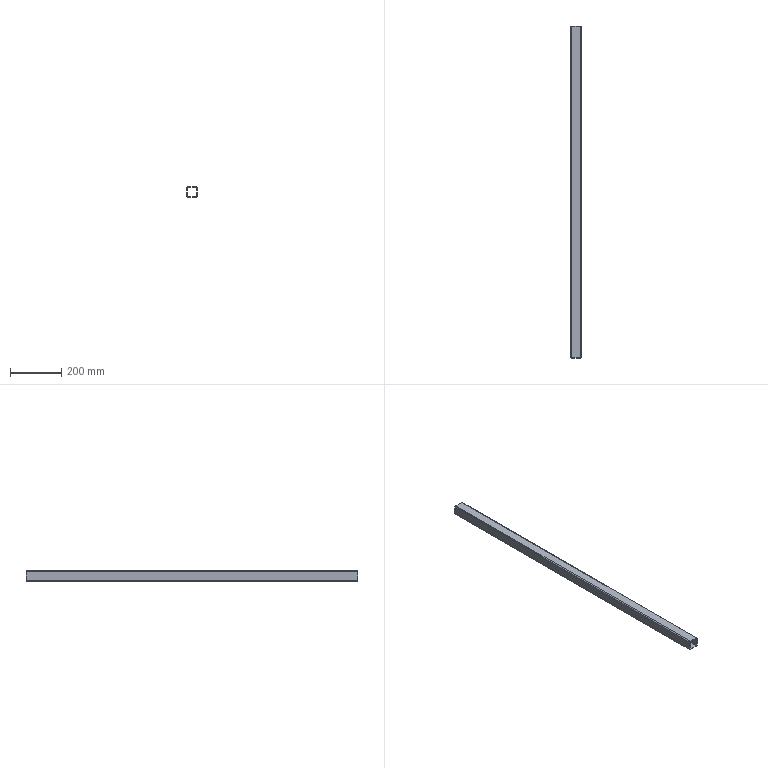Part | STEP file | E3-中转釜护栏7-2立柱主体_Default<As Machined> | 1 solid | 18 faces | box 40 x 1292 x 40 mm | volume 379459 mm3 | plane 10 | cylinder 8 | commonest cylinder face diameters 4 x4 8 x4
STEP:
#1=CARTESIAN_POINT('',(0.,0.,0.));
#2=DIRECTION('',(0.,0.,1.));
#3=DIRECTION('',(1.,0.,0.));
#4=AXIS2_PLACEMENT_3D('',#1,#2,#3);
#5=CARTESIAN_POINT('',(-20.,0.,-16.));
#6=VERTEX_POINT('',#5);
#7=CARTESIAN_POINT('',(-16.,0.,-20.));
#8=VERTEX_POINT('',#7);
#9=CARTESIAN_POINT('',(-16.,0.,-16.));
#10=DIRECTION('',(0.,-1.,0.));
#11=DIRECTION('',(0.,0.,-1.));
#12=AXIS2_PLACEMENT_3D('',#9,#10,#11);
#13=CIRCLE('',#12,4.);
#14=CARTESIAN_POINT('',(-16.,1292.,-16.));
#15=DIRECTION('',(0.,-1.,0.));
#16=DIRECTION('',(0.,0.,1.));
#17=AXIS2_PLACEMENT_3D('',#14,#15,#16);
#18=CYLINDRICAL_SURFACE('',#17,4.);
#19=CARTESIAN_POINT('',(-3.142,1292.));
#20=DIRECTION('',(1.,0.));
#21=VECTOR('',#20,1.);
#22=LINE('',#19,#21);
#23=(GEOMETRIC_REPRESENTATION_CONTEXT(2)PARAMETRIC_REPRESENTATION_CONTEXT()REPRESENTATION_CONTEXT('',''));
#24=DEFINITIONAL_REPRESENTATION('',(#22),#23);
#25=PCURVE('',#18,#24);
#26=CARTESIAN_POINT('',(-16.,0.,-16.));
#27=DIRECTION('',(0.,1.,0.));
#28=DIRECTION('',(0.,0.,-1.));
#29=AXIS2_PLACEMENT_3D('',#26,#27,#28);
#30=PLANE('',#29);
#31=CARTESIAN_POINT('',(4.,0.));
#32=CARTESIAN_POINT('',(4.,-6.928));
#33=CARTESIAN_POINT('',(-2.,-3.464));
#34=CARTESIAN_POINT('',(-8.,0.));
#35=CARTESIAN_POINT('',(-2.,3.464));
#36=CARTESIAN_POINT('',(4.,6.928));
#37=CARTESIAN_POINT('',(4.,0.));
#38=(BOUNDED_CURVE()B_SPLINE_CURVE(2,(#31,#32,#33,#34,#35,#36,#37),.UNSPECIFIED.,.T.,.F.)B_SPLINE_CURVE_WITH_KNOTS((1,2,2,2,2,1),(-2.094,0.,2.094,4.189,6.283,8.378),.UNSPECIFIED.)CURVE()GEOMETRIC_REPRESENTATION_ITEM()RATIONAL_B_SPLINE_CURVE((1.,0.5,1.,0.5,1.,0.5,1.))REPRESENTATION_ITEM(''));
#39=(GEOMETRIC_REPRESENTATION_CONTEXT(2)PARAMETRIC_REPRESENTATION_CONTEXT()REPRESENTATION_CONTEXT('',''));
#40=DEFINITIONAL_REPRESENTATION('',(#38),#39);
#41=PCURVE('',#30,#40);
#42=SURFACE_CURVE('',#13,(#25,#41),.PCURVE_S1.);
#43=EDGE_CURVE('',#6,#8,#42,.T.);
#44=ORIENTED_EDGE('',*,*,#43,.F.);
#45=CARTESIAN_POINT('',(-20.,1292.,-16.));
#46=VERTEX_POINT('',#45);
#47=CARTESIAN_POINT('',(-20.,1292.,-16.));
#48=DIRECTION('',(0.,-1.,0.));
#49=VECTOR('',#48,1.);
#50=LINE('',#47,#49);
#51=CARTESIAN_POINT('',(1.571,0.));
#52=DIRECTION('',(0.,1.));
#53=VECTOR('',#52,1.);
#54=LINE('',#51,#53);
#55=(GEOMETRIC_REPRESENTATION_CONTEXT(2)PARAMETRIC_REPRESENTATION_CONTEXT()REPRESENTATION_CONTEXT('',''));
#56=DEFINITIONAL_REPRESENTATION('',(#54),#55);
#57=PCURVE('',#18,#56);
#58=CARTESIAN_POINT('',(-20.,1292.,-16.));
#59=DIRECTION('',(1.,0.,0.));
#60=DIRECTION('',(0.,0.,1.));
#61=AXIS2_PLACEMENT_3D('',#58,#59,#60);
#62=PLANE('',#61);
#63=CARTESIAN_POINT('',(0.,0.));
#64=DIRECTION('',(0.,1.));
#65=VECTOR('',#64,1.);
#66=LINE('',#63,#65);
#67=(GEOMETRIC_REPRESENTATION_CONTEXT(2)PARAMETRIC_REPRESENTATION_CONTEXT()REPRESENTATION_CONTEXT('',''));
#68=DEFINITIONAL_REPRESENTATION('',(#66),#67);
#69=PCURVE('',#62,#68);
#70=SURFACE_CURVE('',#50,(#57,#69),.PCURVE_S1.);
#71=EDGE_CURVE('',#46,#6,#70,.T.);
#72=ORIENTED_EDGE('',*,*,#71,.F.);
#73=CARTESIAN_POINT('',(-16.,1292.,-20.));
#74=VERTEX_POINT('',#73);
#75=CARTESIAN_POINT('',(-16.,1292.,-16.));
#76=DIRECTION('',(0.,-1.,0.));
#77=DIRECTION('',(0.,0.,-1.));
#78=AXIS2_PLACEMENT_3D('',#75,#76,#77);
#79=CIRCLE('',#78,4.);
#80=CARTESIAN_POINT('',(-3.142,0.));
#81=DIRECTION('',(1.,0.));
#82=VECTOR('',#81,1.);
#83=LINE('',#80,#82);
#84=(GEOMETRIC_REPRESENTATION_CONTEXT(2)PARAMETRIC_REPRESENTATION_CONTEXT()REPRESENTATION_CONTEXT('',''));
#85=DEFINITIONAL_REPRESENTATION('',(#83),#84);
#86=PCURVE('',#18,#85);
#87=CARTESIAN_POINT('',(-16.,1292.,-16.));
#88=DIRECTION('',(0.,1.,0.));
#89=DIRECTION('',(0.,0.,-1.));
#90=AXIS2_PLACEMENT_3D('',#87,#88,#89);
#91=PLANE('',#90);
#92=CARTESIAN_POINT('',(4.,0.));
#93=CARTESIAN_POINT('',(4.,-6.928));
#94=CARTESIAN_POINT('',(-2.,-3.464));
#95=CARTESIAN_POINT('',(-8.,0.));
#96=CARTESIAN_POINT('',(-2.,3.464));
#97=CARTESIAN_POINT('',(4.,6.928));
#98=CARTESIAN_POINT('',(4.,0.));
#99=(BOUNDED_CURVE()B_SPLINE_CURVE(2,(#92,#93,#94,#95,#96,#97,#98),.UNSPECIFIED.,.T.,.F.)B_SPLINE_CURVE_WITH_KNOTS((1,2,2,2,2,1),(-2.094,0.,2.094,4.189,6.283,8.378),.UNSPECIFIED.)CURVE()GEOMETRIC_REPRESENTATION_ITEM()RATIONAL_B_SPLINE_CURVE((1.,0.5,1.,0.5,1.,0.5,1.))REPRESENTATION_ITEM(''));
#100=(GEOMETRIC_REPRESENTATION_CONTEXT(2)PARAMETRIC_REPRESENTATION_CONTEXT()REPRESENTATION_CONTEXT('',''));
#101=DEFINITIONAL_REPRESENTATION('',(#99),#100);
#102=PCURVE('',#91,#101);
#103=SURFACE_CURVE('',#79,(#86,#102),.PCURVE_S1.);
#104=EDGE_CURVE('',#46,#74,#103,.T.);
#105=ORIENTED_EDGE('',*,*,#104,.T.);
#106=CARTESIAN_POINT('',(-16.,1292.,-20.));
#107=DIRECTION('',(0.,-1.,0.));
#108=VECTOR('',#107,1.);
#109=LINE('',#106,#108);
#110=CARTESIAN_POINT('',(3.142,0.));
#111=DIRECTION('',(0.,1.));
#112=VECTOR('',#111,1.);
#113=LINE('',#110,#112);
#114=(GEOMETRIC_REPRESENTATION_CONTEXT(2)PARAMETRIC_REPRESENTATION_CONTEXT()REPRESENTATION_CONTEXT('',''));
#115=DEFINITIONAL_REPRESENTATION('',(#113),#114);
#116=PCURVE('',#18,#115);
#117=CARTESIAN_POINT('',(-16.,1292.,-20.));
#118=DIRECTION('',(0.,0.,1.));
#119=DIRECTION('',(-1.,0.,0.));
#120=AXIS2_PLACEMENT_3D('',#117,#118,#119);
#121=PLANE('',#120);
#122=CARTESIAN_POINT('',(0.,0.));
#123=DIRECTION('',(0.,1.));
#124=VECTOR('',#123,1.);
#125=LINE('',#122,#124);
#126=(GEOMETRIC_REPRESENTATION_CONTEXT(2)PARAMETRIC_REPRESENTATION_CONTEXT()REPRESENTATION_CONTEXT('',''));
#127=DEFINITIONAL_REPRESENTATION('',(#125),#126);
#128=PCURVE('',#121,#127);
#129=SURFACE_CURVE('',#109,(#116,#128),.PCURVE_S1.);
#130=EDGE_CURVE('',#74,#8,#129,.T.);
#131=ORIENTED_EDGE('',*,*,#130,.T.);
#132=EDGE_LOOP('',(#44,#72,#105,#131));
#133=FACE_BOUND('',#132,.T.);
#134=ADVANCED_FACE('',(#133),#18,.T.);
#135=CARTESIAN_POINT('',(16.,0.,-20.));
#136=VERTEX_POINT('',#135);
#137=CARTESIAN_POINT('',(-16.,0.,-20.));
#138=DIRECTION('',(1.,0.,0.));
#139=VECTOR('',#138,1.);
#140=LINE('',#137,#139);
#141=CARTESIAN_POINT('',(0.,1292.));
#142=DIRECTION('',(-1.,0.));
#143=VECTOR('',#142,1.);
#144=LINE('',#141,#143);
#145=(GEOMETRIC_REPRESENTATION_CONTEXT(2)PARAMETRIC_REPRESENTATION_CONTEXT()REPRESENTATION_CONTEXT('',''));
#146=DEFINITIONAL_REPRESENTATION('',(#144),#145);
#147=PCURVE('',#121,#146);
#148=CARTESIAN_POINT('',(4.,0.));
#149=DIRECTION('',(0.,-1.));
#150=VECTOR('',#149,1.);
#151=LINE('',#148,#150);
#152=(GEOMETRIC_REPRESENTATION_CONTEXT(2)PARAMETRIC_REPRESENTATION_CONTEXT()REPRESENTATION_CONTEXT('',''));
#153=DEFINITIONAL_REPRESENTATION('',(#151),#152);
#154=PCURVE('',#30,#153);
#155=SURFACE_CURVE('',#140,(#147,#154),.PCURVE_S1.);
#156=EDGE_CURVE('',#8,#136,#155,.T.);
#157=ORIENTED_EDGE('',*,*,#156,.F.);
#158=ORIENTED_EDGE('',*,*,#130,.F.);
#159=CARTESIAN_POINT('',(16.,1292.,-20.));
#160=VERTEX_POINT('',#159);
#161=CARTESIAN_POINT('',(-16.,1292.,-20.));
#162=DIRECTION('',(1.,0.,0.));
#163=VECTOR('',#162,1.);
#164=LINE('',#161,#163);
#165=CARTESIAN_POINT('',(0.,0.));
#166=DIRECTION('',(-1.,0.));
#167=VECTOR('',#166,1.);
#168=LINE('',#165,#167);
#169=(GEOMETRIC_REPRESENTATION_CONTEXT(2)PARAMETRIC_REPRESENTATION_CONTEXT()REPRESENTATION_CONTEXT('',''));
#170=DEFINITIONAL_REPRESENTATION('',(#168),#169);
#171=PCURVE('',#121,#170);
#172=CARTESIAN_POINT('',(4.,0.));
#173=DIRECTION('',(0.,-1.));
#174=VECTOR('',#173,1.);
#175=LINE('',#172,#174);
#176=(GEOMETRIC_REPRESENTATION_CONTEXT(2)PARAMETRIC_REPRESENTATION_CONTEXT()REPRESENTATION_CONTEXT('',''));
#177=DEFINITIONAL_REPRESENTATION('',(#175),#176);
#178=PCURVE('',#91,#177);
#179=SURFACE_CURVE('',#164,(#171,#178),.PCURVE_S1.);
#180=EDGE_CURVE('',#74,#160,#179,.T.);
#181=ORIENTED_EDGE('',*,*,#180,.T.);
#182=CARTESIAN_POINT('',(16.,1292.,-20.));
#183=DIRECTION('',(0.,-1.,0.));
#184=VECTOR('',#183,1.);
#185=LINE('',#182,#184);
#186=CARTESIAN_POINT('',(-32.,0.));
#187=DIRECTION('',(0.,1.));
#188=VECTOR('',#187,1.);
#189=LINE('',#186,#188);
#190=(GEOMETRIC_REPRESENTATION_CONTEXT(2)PARAMETRIC_REPRESENTATION_CONTEXT()REPRESENTATION_CONTEXT('',''));
#191=DEFINITIONAL_REPRESENTATION('',(#189),#190);
#192=PCURVE('',#121,#191);
#193=CARTESIAN_POINT('',(16.,1292.,-16.));
#194=DIRECTION('',(0.,-1.,0.));
#195=DIRECTION('',(0.,0.,1.));
#196=AXIS2_PLACEMENT_3D('',#193,#194,#195);
#197=CYLINDRICAL_SURFACE('',#196,4.);
#198=CARTESIAN_POINT('',(3.142,0.));
#199=DIRECTION('',(0.,1.));
#200=VECTOR('',#199,1.);
#201=LINE('',#198,#200);
#202=(GEOMETRIC_REPRESENTATION_CONTEXT(2)PARAMETRIC_REPRESENTATION_CONTEXT()REPRESENTATION_CONTEXT('',''));
#203=DEFINITIONAL_REPRESENTATION('',(#201),#202);
#204=PCURVE('',#197,#203);
#205=SURFACE_CURVE('',#185,(#192,#204),.PCURVE_S1.);
#206=EDGE_CURVE('',#160,#136,#205,.T.);
#207=ORIENTED_EDGE('',*,*,#206,.T.);
#208=EDGE_LOOP('',(#157,#158,#181,#207));
#209=FACE_BOUND('',#208,.T.);
#210=ADVANCED_FACE('',(#209),#121,.F.);
#211=CARTESIAN_POINT('',(20.,0.,-16.));
#212=VERTEX_POINT('',#211);
#213=CARTESIAN_POINT('',(16.,0.,-16.));
#214=DIRECTION('',(0.,-1.,0.));
#215=DIRECTION('',(0.,0.,-1.));
#216=AXIS2_PLACEMENT_3D('',#213,#214,#215);
#217=CIRCLE('',#216,4.);
#218=CARTESIAN_POINT('',(3.142,1292.));
#219=DIRECTION('',(1.,0.));
#220=VECTOR('',#219,1.);
#221=LINE('',#218,#220);
#222=(GEOMETRIC_REPRESENTATION_CONTEXT(2)PARAMETRIC_REPRESENTATION_CONTEXT()REPRESENTATION_CONTEXT('',''));
#223=DEFINITIONAL_REPRESENTATION('',(#221),#222);
#224=PCURVE('',#197,#223);
#225=CARTESIAN_POINT('',(4.,-32.));
#226=CARTESIAN_POINT('',(4.,-38.928));
#227=CARTESIAN_POINT('',(-2.,-35.464));
#228=CARTESIAN_POINT('',(-8.,-32.));
#229=CARTESIAN_POINT('',(-2.,-28.536));
#230=CARTESIAN_POINT('',(4.,-25.072));
#231=CARTESIAN_POINT('',(4.,-32.));
#232=(BOUNDED_CURVE()B_SPLINE_CURVE(2,(#225,#226,#227,#228,#229,#230,#231),.UNSPECIFIED.,.T.,.F.)B_SPLINE_CURVE_WITH_KNOTS((1,2,2,2,2,1),(-2.094,0.,2.094,4.189,6.283,8.378),.UNSPECIFIED.)CURVE()GEOMETRIC_REPRESENTATION_ITEM()RATIONAL_B_SPLINE_CURVE((1.,0.5,1.,0.5,1.,0.5,1.))REPRESENTATION_ITEM(''));
#233=(GEOMETRIC_REPRESENTATION_CONTEXT(2)PARAMETRIC_REPRESENTATION_CONTEXT()REPRESENTATION_CONTEXT('',''));
#234=DEFINITIONAL_REPRESENTATION('',(#232),#233);
#235=PCURVE('',#30,#234);
#236=SURFACE_CURVE('',#217,(#224,#235),.PCURVE_S1.);
#237=EDGE_CURVE('',#136,#212,#236,.T.);
#238=ORIENTED_EDGE('',*,*,#237,.F.);
#239=ORIENTED_EDGE('',*,*,#206,.F.);
#240=CARTESIAN_POINT('',(20.,1292.,-16.));
#241=VERTEX_POINT('',#240);
#242=CARTESIAN_POINT('',(16.,1292.,-16.));
#243=DIRECTION('',(0.,-1.,0.));
#244=DIRECTION('',(0.,0.,-1.));
#245=AXIS2_PLACEMENT_3D('',#242,#243,#244);
#246=CIRCLE('',#245,4.);
#247=CARTESIAN_POINT('',(3.142,0.));
#248=DIRECTION('',(1.,0.));
#249=VECTOR('',#248,1.);
#250=LINE('',#247,#249);
#251=(GEOMETRIC_REPRESENTATION_CONTEXT(2)PARAMETRIC_REPRESENTATION_CONTEXT()REPRESENTATION_CONTEXT('',''));
#252=DEFINITIONAL_REPRESENTATION('',(#250),#251);
#253=PCURVE('',#197,#252);
#254=CARTESIAN_POINT('',(4.,-32.));
#255=CARTESIAN_POINT('',(4.,-38.928));
#256=CARTESIAN_POINT('',(-2.,-35.464));
#257=CARTESIAN_POINT('',(-8.,-32.));
#258=CARTESIAN_POINT('',(-2.,-28.536));
#259=CARTESIAN_POINT('',(4.,-25.072));
#260=CARTESIAN_POINT('',(4.,-32.));
#261=(BOUNDED_CURVE()B_SPLINE_CURVE(2,(#254,#255,#256,#257,#258,#259,#260),.UNSPECIFIED.,.T.,.F.)B_SPLINE_CURVE_WITH_KNOTS((1,2,2,2,2,1),(-2.094,0.,2.094,4.189,6.283,8.378),.UNSPECIFIED.)CURVE()GEOMETRIC_REPRESENTATION_ITEM()RATIONAL_B_SPLINE_CURVE((1.,0.5,1.,0.5,1.,0.5,1.))REPRESENTATION_ITEM(''));
#262=(GEOMETRIC_REPRESENTATION_CONTEXT(2)PARAMETRIC_REPRESENTATION_CONTEXT()REPRESENTATION_CONTEXT('',''));
#263=DEFINITIONAL_REPRESENTATION('',(#261),#262);
#264=PCURVE('',#91,#263);
#265=SURFACE_CURVE('',#246,(#253,#264),.PCURVE_S1.);
#266=EDGE_CURVE('',#160,#241,#265,.T.);
#267=ORIENTED_EDGE('',*,*,#266,.T.);
#268=CARTESIAN_POINT('',(20.,1292.,-16.));
#269=DIRECTION('',(0.,-1.,0.));
#270=VECTOR('',#269,1.);
#271=LINE('',#268,#270);
#272=CARTESIAN_POINT('',(4.712,0.));
#273=DIRECTION('',(0.,1.));
#274=VECTOR('',#273,1.);
#275=LINE('',#272,#274);
#276=(GEOMETRIC_REPRESENTATION_CONTEXT(2)PARAMETRIC_REPRESENTATION_CONTEXT()REPRESENTATION_CONTEXT('',''));
#277=DEFINITIONAL_REPRESENTATION('',(#275),#276);
#278=PCURVE('',#197,#277);
#279=CARTESIAN_POINT('',(20.,1292.,16.));
#280=DIRECTION('',(-1.,0.,0.));
#281=DIRECTION('',(0.,0.,-1.));
#282=AXIS2_PLACEMENT_3D('',#279,#280,#281);
#283=PLANE('',#282);
#284=CARTESIAN_POINT('',(32.,0.));
#285=DIRECTION('',(0.,1.));
#286=VECTOR('',#285,1.);
#287=LINE('',#284,#286);
#288=(GEOMETRIC_REPRESENTATION_CONTEXT(2)PARAMETRIC_REPRESENTATION_CONTEXT()REPRESENTATION_CONTEXT('',''));
#289=DEFINITIONAL_REPRESENTATION('',(#287),#288);
#290=PCURVE('',#283,#289);
#291=SURFACE_CURVE('',#271,(#278,#290),.PCURVE_S1.);
#292=EDGE_CURVE('',#241,#212,#291,.T.);
#293=ORIENTED_EDGE('',*,*,#292,.T.);
#294=EDGE_LOOP('',(#238,#239,#267,#293));
#295=FACE_BOUND('',#294,.T.);
#296=ADVANCED_FACE('',(#295),#197,.T.);
#297=CARTESIAN_POINT('',(20.,0.,16.));
#298=VERTEX_POINT('',#297);
#299=CARTESIAN_POINT('',(20.,0.,16.));
#300=DIRECTION('',(0.,0.,1.));
#301=VECTOR('',#300,1.);
#302=LINE('',#299,#301);
#303=CARTESIAN_POINT('',(0.,1292.));
#304=DIRECTION('',(-1.,0.));
#305=VECTOR('',#304,1.);
#306=LINE('',#303,#305);
#307=(GEOMETRIC_REPRESENTATION_CONTEXT(2)PARAMETRIC_REPRESENTATION_CONTEXT()REPRESENTATION_CONTEXT('',''));
#308=DEFINITIONAL_REPRESENTATION('',(#306),#307);
#309=PCURVE('',#283,#308);
#310=CARTESIAN_POINT('',(-32.,-36.));
#311=DIRECTION('',(-1.,0.));
#312=VECTOR('',#311,1.);
#313=LINE('',#310,#312);
#314=(GEOMETRIC_REPRESENTATION_CONTEXT(2)PARAMETRIC_REPRESENTATION_CONTEXT()REPRESENTATION_CONTEXT('',''));
#315=DEFINITIONAL_REPRESENTATION('',(#313),#314);
#316=PCURVE('',#30,#315);
#317=SURFACE_CURVE('',#302,(#309,#316),.PCURVE_S1.);
#318=EDGE_CURVE('',#212,#298,#317,.T.);
#319=ORIENTED_EDGE('',*,*,#318,.F.);
#320=ORIENTED_EDGE('',*,*,#292,.F.);
#321=CARTESIAN_POINT('',(20.,1292.,16.));
#322=VERTEX_POINT('',#321);
#323=CARTESIAN_POINT('',(20.,1292.,16.));
#324=DIRECTION('',(0.,0.,1.));
#325=VECTOR('',#324,1.);
#326=LINE('',#323,#325);
#327=CARTESIAN_POINT('',(0.,0.));
#328=DIRECTION('',(-1.,0.));
#329=VECTOR('',#328,1.);
#330=LINE('',#327,#329);
#331=(GEOMETRIC_REPRESENTATION_CONTEXT(2)PARAMETRIC_REPRESENTATION_CONTEXT()REPRESENTATION_CONTEXT('',''));
#332=DEFINITIONAL_REPRESENTATION('',(#330),#331);
#333=PCURVE('',#283,#332);
#334=CARTESIAN_POINT('',(-32.,-36.));
#335=DIRECTION('',(-1.,0.));
#336=VECTOR('',#335,1.);
#337=LINE('',#334,#336);
#338=(GEOMETRIC_REPRESENTATION_CONTEXT(2)PARAMETRIC_REPRESENTATION_CONTEXT()REPRESENTATION_CONTEXT('',''));
#339=DEFINITIONAL_REPRESENTATION('',(#337),#338);
#340=PCURVE('',#91,#339);
#341=SURFACE_CURVE('',#326,(#333,#340),.PCURVE_S1.);
#342=EDGE_CURVE('',#241,#322,#341,.T.);
#343=ORIENTED_EDGE('',*,*,#342,.T.);
#344=CARTESIAN_POINT('',(20.,1292.,16.));
#345=DIRECTION('',(0.,-1.,0.));
#346=VECTOR('',#345,1.);
#347=LINE('',#344,#346);
#348=CARTESIAN_POINT('',(0.,0.));
#349=DIRECTION('',(0.,1.));
#350=VECTOR('',#349,1.);
#351=LINE('',#348,#350);
#352=(GEOMETRIC_REPRESENTATION_CONTEXT(2)PARAMETRIC_REPRESENTATION_CONTEXT()REPRESENTATION_CONTEXT('',''));
#353=DEFINITIONAL_REPRESENTATION('',(#351),#352);
#354=PCURVE('',#283,#353);
#355=CARTESIAN_POINT('',(16.,1292.,16.));
#356=DIRECTION('',(0.,-1.,0.));
#357=DIRECTION('',(0.,0.,1.));
#358=AXIS2_PLACEMENT_3D('',#355,#356,#357);
#359=CYLINDRICAL_SURFACE('',#358,4.);
#360=CARTESIAN_POINT('',(4.712,0.));
#361=DIRECTION('',(0.,1.));
#362=VECTOR('',#361,1.);
#363=LINE('',#360,#362);
#364=(GEOMETRIC_REPRESENTATION_CONTEXT(2)PARAMETRIC_REPRESENTATION_CONTEXT()REPRESENTATION_CONTEXT('',''));
#365=DEFINITIONAL_REPRESENTATION('',(#363),#364);
#366=PCURVE('',#359,#365);
#367=SURFACE_CURVE('',#347,(#354,#366),.PCURVE_S1.);
#368=EDGE_CURVE('',#322,#298,#367,.T.);
#369=ORIENTED_EDGE('',*,*,#368,.T.);
#370=EDGE_LOOP('',(#319,#320,#343,#369));
#371=FACE_BOUND('',#370,.T.);
#372=ADVANCED_FACE('',(#371),#283,.F.);
#373=CARTESIAN_POINT('',(16.,0.,20.));
#374=VERTEX_POINT('',#373);
#375=CARTESIAN_POINT('',(16.,0.,16.));
#376=DIRECTION('',(0.,-1.,0.));
#377=DIRECTION('',(0.,0.,-1.));
#378=AXIS2_PLACEMENT_3D('',#375,#376,#377);
#379=CIRCLE('',#378,4.);
#380=CARTESIAN_POINT('',(3.142,1292.));
#381=DIRECTION('',(1.,0.));
#382=VECTOR('',#381,1.);
#383=LINE('',#380,#382);
#384=(GEOMETRIC_REPRESENTATION_CONTEXT(2)PARAMETRIC_REPRESENTATION_CONTEXT()REPRESENTATION_CONTEXT('',''));
#385=DEFINITIONAL_REPRESENTATION('',(#383),#384);
#386=PCURVE('',#359,#385);
#387=CARTESIAN_POINT('',(-28.,-32.));
#388=CARTESIAN_POINT('',(-28.,-38.928));
#389=CARTESIAN_POINT('',(-34.,-35.464));
#390=CARTESIAN_POINT('',(-40.,-32.));
#391=CARTESIAN_POINT('',(-34.,-28.536));
#392=CARTESIAN_POINT('',(-28.,-25.072));
#393=CARTESIAN_POINT('',(-28.,-32.));
#394=(BOUNDED_CURVE()B_SPLINE_CURVE(2,(#387,#388,#389,#390,#391,#392,#393),.UNSPECIFIED.,.T.,.F.)B_SPLINE_CURVE_WITH_KNOTS((1,2,2,2,2,1),(-2.094,0.,2.094,4.189,6.283,8.378),.UNSPECIFIED.)CURVE()GEOMETRIC_REPRESENTATION_ITEM()RATIONAL_B_SPLINE_CURVE((1.,0.5,1.,0.5,1.,0.5,1.))REPRESENTATION_ITEM(''));
#395=(GEOMETRIC_REPRESENTATION_CONTEXT(2)PARAMETRIC_REPRESENTATION_CONTEXT()REPRESENTATION_CONTEXT('',''));
#396=DEFINITIONAL_REPRESENTATION('',(#394),#395);
#397=PCURVE('',#30,#396);
#398=SURFACE_CURVE('',#379,(#386,#397),.PCURVE_S1.);
#399=EDGE_CURVE('',#298,#374,#398,.T.);
#400=ORIENTED_EDGE('',*,*,#399,.F.);
#401=ORIENTED_EDGE('',*,*,#368,.F.);
#402=CARTESIAN_POINT('',(16.,1292.,20.));
#403=VERTEX_POINT('',#402);
#404=CARTESIAN_POINT('',(16.,1292.,16.));
#405=DIRECTION('',(0.,-1.,0.));
#406=DIRECTION('',(0.,0.,-1.));
#407=AXIS2_PLACEMENT_3D('',#404,#405,#406);
#408=CIRCLE('',#407,4.);
#409=CARTESIAN_POINT('',(3.142,0.));
#410=DIRECTION('',(1.,0.));
#411=VECTOR('',#410,1.);
#412=LINE('',#409,#411);
#413=(GEOMETRIC_REPRESENTATION_CONTEXT(2)PARAMETRIC_REPRESENTATION_CONTEXT()REPRESENTATION_CONTEXT('',''));
#414=DEFINITIONAL_REPRESENTATION('',(#412),#413);
#415=PCURVE('',#359,#414);
#416=CARTESIAN_POINT('',(-28.,-32.));
#417=CARTESIAN_POINT('',(-28.,-38.928));
#418=CARTESIAN_POINT('',(-34.,-35.464));
#419=CARTESIAN_POINT('',(-40.,-32.));
#420=CARTESIAN_POINT('',(-34.,-28.536));
#421=CARTESIAN_POINT('',(-28.,-25.072));
#422=CARTESIAN_POINT('',(-28.,-32.));
#423=(BOUNDED_CURVE()B_SPLINE_CURVE(2,(#416,#417,#418,#419,#420,#421,#422),.UNSPECIFIED.,.T.,.F.)B_SPLINE_CURVE_WITH_KNOTS((1,2,2,2,2,1),(-2.094,0.,2.094,4.189,6.283,8.378),.UNSPECIFIED.)CURVE()GEOMETRIC_REPRESENTATION_ITEM()RATIONAL_B_SPLINE_CURVE((1.,0.5,1.,0.5,1.,0.5,1.))REPRESENTATION_ITEM(''));
#424=(GEOMETRIC_REPRESENTATION_CONTEXT(2)PARAMETRIC_REPRESENTATION_CONTEXT()REPRESENTATION_CONTEXT('',''));
#425=DEFINITIONAL_REPRESENTATION('',(#423),#424);
#426=PCURVE('',#91,#425);
#427=SURFACE_CURVE('',#408,(#415,#426),.PCURVE_S1.);
#428=EDGE_CURVE('',#322,#403,#427,.T.);
#429=ORIENTED_EDGE('',*,*,#428,.T.);
#430=CARTESIAN_POINT('',(16.,1292.,20.));
#431=DIRECTION('',(0.,-1.,0.));
#432=VECTOR('',#431,1.);
#433=LINE('',#430,#432);
#434=CARTESIAN_POINT('',(6.283,0.));
#435=DIRECTION('',(0.,1.));
#436=VECTOR('',#435,1.);
#437=LINE('',#434,#436);
#438=(GEOMETRIC_REPRESENTATION_CONTEXT(2)PARAMETRIC_REPRESENTATION_CONTEXT()REPRESENTATION_CONTEXT('',''));
#439=DEFINITIONAL_REPRESENTATION('',(#437),#438);
#440=PCURVE('',#359,#439);
#441=CARTESIAN_POINT('',(16.,1292.,20.));
#442=DIRECTION('',(0.,0.,-1.));
#443=DIRECTION('',(1.,0.,0.));
#444=AXIS2_PLACEMENT_3D('',#441,#442,#443);
#445=PLANE('',#444);
#446=CARTESIAN_POINT('',(0.,0.));
#447=DIRECTION('',(0.,1.));
#448=VECTOR('',#447,1.);
#449=LINE('',#446,#448);
#450=(GEOMETRIC_REPRESENTATION_CONTEXT(2)PARAMETRIC_REPRESENTATION_CONTEXT()REPRESENTATION_CONTEXT('',''));
#451=DEFINITIONAL_REPRESENTATION('',(#449),#450);
#452=PCURVE('',#445,#451);
#453=SURFACE_CURVE('',#433,(#440,#452),.PCURVE_S1.);
#454=EDGE_CURVE('',#403,#374,#453,.T.);
#455=ORIENTED_EDGE('',*,*,#454,.T.);
#456=EDGE_LOOP('',(#400,#401,#429,#455));
#457=FACE_BOUND('',#456,.T.);
#458=ADVANCED_FACE('',(#457),#359,.T.);
#459=CARTESIAN_POINT('',(-16.,0.,20.));
#460=VERTEX_POINT('',#459);
#461=CARTESIAN_POINT('',(16.,0.,20.));
#462=DIRECTION('',(-1.,0.,0.));
#463=VECTOR('',#462,1.);
#464=LINE('',#461,#463);
#465=CARTESIAN_POINT('',(0.,1292.));
#466=DIRECTION('',(-1.,0.));
#467=VECTOR('',#466,1.);
#468=LINE('',#465,#467);
#469=(GEOMETRIC_REPRESENTATION_CONTEXT(2)PARAMETRIC_REPRESENTATION_CONTEXT()REPRESENTATION_CONTEXT('',''));
#470=DEFINITIONAL_REPRESENTATION('',(#468),#469);
#471=PCURVE('',#445,#470);
#472=CARTESIAN_POINT('',(-36.,-32.));
#473=DIRECTION('',(0.,1.));
#474=VECTOR('',#473,1.);
#475=LINE('',#472,#474);
#476=(GEOMETRIC_REPRESENTATION_CONTEXT(2)PARAMETRIC_REPRESENTATION_CONTEXT()REPRESENTATION_CONTEXT('',''));
#477=DEFINITIONAL_REPRESENTATION('',(#475),#476);
#478=PCURVE('',#30,#477);
#479=SURFACE_CURVE('',#464,(#471,#478),.PCURVE_S1.);
#480=EDGE_CURVE('',#374,#460,#479,.T.);
#481=ORIENTED_EDGE('',*,*,#480,.F.);
#482=ORIENTED_EDGE('',*,*,#454,.F.);
#483=CARTESIAN_POINT('',(-16.,1292.,20.));
#484=VERTEX_POINT('',#483);
#485=CARTESIAN_POINT('',(16.,1292.,20.));
#486=DIRECTION('',(-1.,0.,0.));
#487=VECTOR('',#486,1.);
#488=LINE('',#485,#487);
#489=CARTESIAN_POINT('',(0.,0.));
#490=DIRECTION('',(-1.,0.));
#491=VECTOR('',#490,1.);
#492=LINE('',#489,#491);
#493=(GEOMETRIC_REPRESENTATION_CONTEXT(2)PARAMETRIC_REPRESENTATION_CONTEXT()REPRESENTATION_CONTEXT('',''));
#494=DEFINITIONAL_REPRESENTATION('',(#492),#493);
#495=PCURVE('',#445,#494);
#496=CARTESIAN_POINT('',(-36.,-32.));
#497=DIRECTION('',(0.,1.));
#498=VECTOR('',#497,1.);
#499=LINE('',#496,#498);
#500=(GEOMETRIC_REPRESENTATION_CONTEXT(2)PARAMETRIC_REPRESENTATION_CONTEXT()REPRESENTATION_CONTEXT('',''));
#501=DEFINITIONAL_REPRESENTATION('',(#499),#500);
#502=PCURVE('',#91,#501);
#503=SURFACE_CURVE('',#488,(#495,#502),.PCURVE_S1.);
#504=EDGE_CURVE('',#403,#484,#503,.T.);
#505=ORIENTED_EDGE('',*,*,#504,.T.);
#506=CARTESIAN_POINT('',(-16.,1292.,20.));
#507=DIRECTION('',(0.,-1.,0.));
#508=VECTOR('',#507,1.);
#509=LINE('',#506,#508);
#510=CARTESIAN_POINT('',(-32.,0.));
#511=DIRECTION('',(0.,1.));
#512=VECTOR('',#511,1.);
#513=LINE('',#510,#512);
#514=(GEOMETRIC_REPRESENTATION_CONTEXT(2)PARAMETRIC_REPRESENTATION_CONTEXT()REPRESENTATION_CONTEXT('',''));
#515=DEFINITIONAL_REPRESENTATION('',(#513),#514);
#516=PCURVE('',#445,#515);
#517=CARTESIAN_POINT('',(-16.,1292.,16.));
#518=DIRECTION('',(0.,-1.,0.));
#519=DIRECTION('',(0.,0.,1.));
#520=AXIS2_PLACEMENT_3D('',#517,#518,#519);
#521=CYLINDRICAL_SURFACE('',#520,4.);
#522=CARTESIAN_POINT('',(0.,0.));
#523=DIRECTION('',(0.,1.));
#524=VECTOR('',#523,1.);
#525=LINE('',#522,#524);
#526=(GEOMETRIC_REPRESENTATION_CONTEXT(2)PARAMETRIC_REPRESENTATION_CONTEXT()REPRESENTATION_CONTEXT('',''));
#527=DEFINITIONAL_REPRESENTATION('',(#525),#526);
#528=PCURVE('',#521,#527);
#529=SURFACE_CURVE('',#509,(#516,#528),.PCURVE_S1.);
#530=EDGE_CURVE('',#484,#460,#529,.T.);
#531=ORIENTED_EDGE('',*,*,#530,.T.);
#532=EDGE_LOOP('',(#481,#482,#505,#531));
#533=FACE_BOUND('',#532,.T.);
#534=ADVANCED_FACE('',(#533),#445,.F.);
#535=CARTESIAN_POINT('',(-20.,0.,16.));
#536=VERTEX_POINT('',#535);
#537=CARTESIAN_POINT('',(-16.,0.,16.));
#538=DIRECTION('',(0.,-1.,0.));
#539=DIRECTION('',(0.,0.,-1.));
#540=AXIS2_PLACEMENT_3D('',#537,#538,#539);
#541=CIRCLE('',#540,4.);
#542=CARTESIAN_POINT('',(-3.142,1292.));
#543=DIRECTION('',(1.,0.));
#544=VECTOR('',#543,1.);
#545=LINE('',#542,#544);
#546=(GEOMETRIC_REPRESENTATION_CONTEXT(2)PARAMETRIC_REPRESENTATION_CONTEXT()REPRESENTATION_CONTEXT('',''));
#547=DEFINITIONAL_REPRESENTATION('',(#545),#546);
#548=PCURVE('',#521,#547);
#549=CARTESIAN_POINT('',(-28.,0.));
#550=CARTESIAN_POINT('',(-28.,-6.928));
#551=CARTESIAN_POINT('',(-34.,-3.464));
#552=CARTESIAN_POINT('',(-40.,0.));
#553=CARTESIAN_POINT('',(-34.,3.464));
#554=CARTESIAN_POINT('',(-28.,6.928));
#555=CARTESIAN_POINT('',(-28.,0.));
#556=(BOUNDED_CURVE()B_SPLINE_CURVE(2,(#549,#550,#551,#552,#553,#554,#555),.UNSPECIFIED.,.T.,.F.)B_SPLINE_CURVE_WITH_KNOTS((1,2,2,2,2,1),(-2.094,0.,2.094,4.189,6.283,8.378),.UNSPECIFIED.)CURVE()GEOMETRIC_REPRESENTATION_ITEM()RATIONAL_B_SPLINE_CURVE((1.,0.5,1.,0.5,1.,0.5,1.))REPRESENTATION_ITEM(''));
#557=(GEOMETRIC_REPRESENTATION_CONTEXT(2)PARAMETRIC_REPRESENTATION_CONTEXT()REPRESENTATION_CONTEXT('',''));
#558=DEFINITIONAL_REPRESENTATION('',(#556),#557);
#559=PCURVE('',#30,#558);
#560=SURFACE_CURVE('',#541,(#548,#559),.PCURVE_S1.);
#561=EDGE_CURVE('',#460,#536,#560,.T.);
#562=ORIENTED_EDGE('',*,*,#561,.F.);
#563=ORIENTED_EDGE('',*,*,#530,.F.);
#564=CARTESIAN_POINT('',(-20.,1292.,16.));
#565=VERTEX_POINT('',#564);
#566=CARTESIAN_POINT('',(-16.,1292.,16.));
#567=DIRECTION('',(0.,-1.,0.));
#568=DIRECTION('',(0.,0.,-1.));
#569=AXIS2_PLACEMENT_3D('',#566,#567,#568);
#570=CIRCLE('',#569,4.);
#571=CARTESIAN_POINT('',(-3.142,0.));
#572=DIRECTION('',(1.,0.));
#573=VECTOR('',#572,1.);
#574=LINE('',#571,#573);
#575=(GEOMETRIC_REPRESENTATION_CONTEXT(2)PARAMETRIC_REPRESENTATION_CONTEXT()REPRESENTATION_CONTEXT('',''));
#576=DEFINITIONAL_REPRESENTATION('',(#574),#575);
#577=PCURVE('',#521,#576);
#578=CARTESIAN_POINT('',(-28.,0.));
#579=CARTESIAN_POINT('',(-28.,-6.928));
#580=CARTESIAN_POINT('',(-34.,-3.464));
#581=CARTESIAN_POINT('',(-40.,0.));
#582=CARTESIAN_POINT('',(-34.,3.464));
#583=CARTESIAN_POINT('',(-28.,6.928));
#584=CARTESIAN_POINT('',(-28.,0.));
#585=(BOUNDED_CURVE()B_SPLINE_CURVE(2,(#578,#579,#580,#581,#582,#583,#584),.UNSPECIFIED.,.T.,.F.)B_SPLINE_CURVE_WITH_KNOTS((1,2,2,2,2,1),(-2.094,0.,2.094,4.189,6.283,8.378),.UNSPECIFIED.)CURVE()GEOMETRIC_REPRESENTATION_ITEM()RATIONAL_B_SPLINE_CURVE((1.,0.5,1.,0.5,1.,0.5,1.))REPRESENTATION_ITEM(''));
#586=(GEOMETRIC_REPRESENTATION_CONTEXT(2)PARAMETRIC_REPRESENTATION_CONTEXT()REPRESENTATION_CONTEXT('',''));
#587=DEFINITIONAL_REPRESENTATION('',(#585),#586);
#588=PCURVE('',#91,#587);
#589=SURFACE_CURVE('',#570,(#577,#588),.PCURVE_S1.);
#590=EDGE_CURVE('',#484,#565,#589,.T.);
#591=ORIENTED_EDGE('',*,*,#590,.T.);
#592=CARTESIAN_POINT('',(-20.,1292.,16.));
#593=DIRECTION('',(0.,-1.,0.));
#594=VECTOR('',#593,1.);
#595=LINE('',#592,#594);
#596=CARTESIAN_POINT('',(1.571,0.));
#597=DIRECTION('',(0.,1.));
#598=VECTOR('',#597,1.);
#599=LINE('',#596,#598);
#600=(GEOMETRIC_REPRESENTATION_CONTEXT(2)PARAMETRIC_REPRESENTATION_CONTEXT()REPRESENTATION_CONTEXT('',''));
#601=DEFINITIONAL_REPRESENTATION('',(#599),#600);
#602=PCURVE('',#521,#601);
#603=CARTESIAN_POINT('',(32.,0.));
#604=DIRECTION('',(0.,1.));
#605=VECTOR('',#604,1.);
#606=LINE('',#603,#605);
#607=(GEOMETRIC_REPRESENTATION_CONTEXT(2)PARAMETRIC_REPRESENTATION_CONTEXT()REPRESENTATION_CONTEXT('',''));
#608=DEFINITIONAL_REPRESENTATION('',(#606),#607);
#609=PCURVE('',#62,#608);
#610=SURFACE_CURVE('',#595,(#602,#609),.PCURVE_S1.);
#611=EDGE_CURVE('',#565,#536,#610,.T.);
#612=ORIENTED_EDGE('',*,*,#611,.T.);
#613=EDGE_LOOP('',(#562,#563,#591,#612));
#614=FACE_BOUND('',#613,.T.);
#615=ADVANCED_FACE('',(#614),#521,.T.);
#616=CARTESIAN_POINT('',(16.,1292.,-18.));
#617=VERTEX_POINT('',#616);
#618=CARTESIAN_POINT('',(16.,0.,-18.));
#619=VERTEX_POINT('',#618);
#620=CARTESIAN_POINT('',(16.,1292.,-18.));
#621=DIRECTION('',(0.,-1.,0.));
#622=VECTOR('',#621,1.);
#623=LINE('',#620,#622);
#624=CARTESIAN_POINT('',(16.,1292.,-16.));
#625=DIRECTION('',(0.,-1.,0.));
#626=DIRECTION('',(0.,0.,1.));
#627=AXIS2_PLACEMENT_3D('',#624,#625,#626);
#628=CYLINDRICAL_SURFACE('',#627,2.);
#629=CARTESIAN_POINT('',(3.142,0.));
#630=DIRECTION('',(0.,1.));
#631=VECTOR('',#630,1.);
#632=LINE('',#629,#631);
#633=(GEOMETRIC_REPRESENTATION_CONTEXT(2)PARAMETRIC_REPRESENTATION_CONTEXT()REPRESENTATION_CONTEXT('',''));
#634=DEFINITIONAL_REPRESENTATION('',(#632),#633);
#635=PCURVE('',#628,#634);
#636=CARTESIAN_POINT('',(-16.,1292.,-18.));
#637=DIRECTION('',(0.,0.,1.));
#638=DIRECTION('',(-1.,0.,0.));
#639=AXIS2_PLACEMENT_3D('',#636,#637,#638);
#640=PLANE('',#639);
#641=CARTESIAN_POINT('',(-32.,0.));
#642=DIRECTION('',(0.,1.));
#643=VECTOR('',#642,1.);
#644=LINE('',#641,#643);
#645=(GEOMETRIC_REPRESENTATION_CONTEXT(2)PARAMETRIC_REPRESENTATION_CONTEXT()REPRESENTATION_CONTEXT('',''));
#646=DEFINITIONAL_REPRESENTATION('',(#644),#645);
#647=PCURVE('',#640,#646);
#648=SURFACE_CURVE('',#623,(#635,#647),.PCURVE_S1.);
#649=EDGE_CURVE('',#617,#619,#648,.T.);
#650=ORIENTED_EDGE('',*,*,#649,.F.);
#651=CARTESIAN_POINT('',(18.,1292.,-16.));
#652=VERTEX_POINT('',#651);
#653=CARTESIAN_POINT('',(16.,1292.,-16.));
#654=DIRECTION('',(0.,-1.,0.));
#655=DIRECTION('',(0.,0.,-1.));
#656=AXIS2_PLACEMENT_3D('',#653,#654,#655);
#657=CIRCLE('',#656,2.);
#658=CARTESIAN_POINT('',(3.142,0.));
#659=DIRECTION('',(1.,0.));
#660=VECTOR('',#659,1.);
#661=LINE('',#658,#660);
#662=(GEOMETRIC_REPRESENTATION_CONTEXT(2)PARAMETRIC_REPRESENTATION_CONTEXT()REPRESENTATION_CONTEXT('',''));
#663=DEFINITIONAL_REPRESENTATION('',(#661),#662);
#664=PCURVE('',#628,#663);
#665=CARTESIAN_POINT('',(2.,-32.));
#666=CARTESIAN_POINT('',(2.,-35.464));
#667=CARTESIAN_POINT('',(-1.,-33.732));
#668=CARTESIAN_POINT('',(-4.,-32.));
#669=CARTESIAN_POINT('',(-1.,-30.268));
#670=CARTESIAN_POINT('',(2.,-28.536));
#671=CARTESIAN_POINT('',(2.,-32.));
#672=(BOUNDED_CURVE()B_SPLINE_CURVE(2,(#665,#666,#667,#668,#669,#670,#671),.UNSPECIFIED.,.T.,.F.)B_SPLINE_CURVE_WITH_KNOTS((1,2,2,2,2,1),(-2.094,0.,2.094,4.189,6.283,8.378),.UNSPECIFIED.)CURVE()GEOMETRIC_REPRESENTATION_ITEM()RATIONAL_B_SPLINE_CURVE((1.,0.5,1.,0.5,1.,0.5,1.))REPRESENTATION_ITEM(''));
#673=(GEOMETRIC_REPRESENTATION_CONTEXT(2)PARAMETRIC_REPRESENTATION_CONTEXT()REPRESENTATION_CONTEXT('',''));
#674=DEFINITIONAL_REPRESENTATION('',(#672),#673);
#675=PCURVE('',#91,#674);
#676=SURFACE_CURVE('',#657,(#664,#675),.PCURVE_S1.);
#677=EDGE_CURVE('',#617,#652,#676,.T.);
#678=ORIENTED_EDGE('',*,*,#677,.T.);
#679=CARTESIAN_POINT('',(18.,0.,-16.));
#680=VERTEX_POINT('',#679);
#681=CARTESIAN_POINT('',(18.,1292.,-16.));
#682=DIRECTION('',(0.,-1.,0.));
#683=VECTOR('',#682,1.);
#684=LINE('',#681,#683);
#685=CARTESIAN_POINT('',(4.712,0.));
#686=DIRECTION('',(0.,1.));
#687=VECTOR('',#686,1.);
#688=LINE('',#685,#687);
#689=(GEOMETRIC_REPRESENTATION_CONTEXT(2)PARAMETRIC_REPRESENTATION_CONTEXT()REPRESENTATION_CONTEXT('',''));
#690=DEFINITIONAL_REPRESENTATION('',(#688),#689);
#691=PCURVE('',#628,#690);
#692=CARTESIAN_POINT('',(18.,1292.,16.));
#693=DIRECTION('',(-1.,0.,0.));
#694=DIRECTION('',(0.,0.,-1.));
#695=AXIS2_PLACEMENT_3D('',#692,#693,#694);
#696=PLANE('',#695);
#697=CARTESIAN_POINT('',(32.,0.));
#698=DIRECTION('',(0.,1.));
#699=VECTOR('',#698,1.);
#700=LINE('',#697,#699);
#701=(GEOMETRIC_REPRESENTATION_CONTEXT(2)PARAMETRIC_REPRESENTATION_CONTEXT()REPRESENTATION_CONTEXT('',''));
#702=DEFINITIONAL_REPRESENTATION('',(#700),#701);
#703=PCURVE('',#696,#702);
#704=SURFACE_CURVE('',#684,(#691,#703),.PCURVE_S1.);
#705=EDGE_CURVE('',#652,#680,#704,.T.);
#706=ORIENTED_EDGE('',*,*,#705,.T.);
#707=CARTESIAN_POINT('',(16.,0.,-16.));
#708=DIRECTION('',(0.,-1.,0.));
#709=DIRECTION('',(0.,0.,-1.));
#710=AXIS2_PLACEMENT_3D('',#707,#708,#709);
#711=CIRCLE('',#710,2.);
#712=CARTESIAN_POINT('',(3.142,1292.));
#713=DIRECTION('',(1.,0.));
#714=VECTOR('',#713,1.);
#715=LINE('',#712,#714);
#716=(GEOMETRIC_REPRESENTATION_CONTEXT(2)PARAMETRIC_REPRESENTATION_CONTEXT()REPRESENTATION_CONTEXT('',''));
#717=DEFINITIONAL_REPRESENTATION('',(#715),#716);
#718=PCURVE('',#628,#717);
#719=CARTESIAN_POINT('',(2.,-32.));
#720=CARTESIAN_POINT('',(2.,-35.464));
#721=CARTESIAN_POINT('',(-1.,-33.732));
#722=CARTESIAN_POINT('',(-4.,-32.));
#723=CARTESIAN_POINT('',(-1.,-30.268));
#724=CARTESIAN_POINT('',(2.,-28.536));
#725=CARTESIAN_POINT('',(2.,-32.));
#726=(BOUNDED_CURVE()B_SPLINE_CURVE(2,(#719,#720,#721,#722,#723,#724,#725),.UNSPECIFIED.,.T.,.F.)B_SPLINE_CURVE_WITH_KNOTS((1,2,2,2,2,1),(-2.094,0.,2.094,4.189,6.283,8.378),.UNSPECIFIED.)CURVE()GEOMETRIC_REPRESENTATION_ITEM()RATIONAL_B_SPLINE_CURVE((1.,0.5,1.,0.5,1.,0.5,1.))REPRESENTATION_ITEM(''));
#727=(GEOMETRIC_REPRESENTATION_CONTEXT(2)PARAMETRIC_REPRESENTATION_CONTEXT()REPRESENTATION_CONTEXT('',''));
#728=DEFINITIONAL_REPRESENTATION('',(#726),#727);
#729=PCURVE('',#30,#728);
#730=SURFACE_CURVE('',#711,(#718,#729),.PCURVE_S1.);
#731=EDGE_CURVE('',#619,#680,#730,.T.);
#732=ORIENTED_EDGE('',*,*,#731,.F.);
#733=EDGE_LOOP('',(#650,#678,#706,#732));
#734=FACE_BOUND('',#733,.F.);
#735=ADVANCED_FACE('',(#734),#628,.F.);
#736=CARTESIAN_POINT('',(-16.,0.,-18.));
#737=VERTEX_POINT('',#736);
#738=CARTESIAN_POINT('',(-16.,0.,-18.));
#739=DIRECTION('',(1.,0.,0.));
#740=VECTOR('',#739,1.);
#741=LINE('',#738,#740);
#742=CARTESIAN_POINT('',(0.,1292.));
#743=DIRECTION('',(-1.,0.));
#744=VECTOR('',#743,1.);
#745=LINE('',#742,#744);
#746=(GEOMETRIC_REPRESENTATION_CONTEXT(2)PARAMETRIC_REPRESENTATION_CONTEXT()REPRESENTATION_CONTEXT('',''));
#747=DEFINITIONAL_REPRESENTATION('',(#745),#746);
#748=PCURVE('',#640,#747);
#749=CARTESIAN_POINT('',(2.,0.));
#750=DIRECTION('',(0.,-1.));
#751=VECTOR('',#750,1.);
#752=LINE('',#749,#751);
#753=(GEOMETRIC_REPRESENTATION_CONTEXT(2)PARAMETRIC_REPRESENTATION_CONTEXT()REPRESENTATION_CONTEXT('',''));
#754=DEFINITIONAL_REPRESENTATION('',(#752),#753);
#755=PCURVE('',#30,#754);
#756=SURFACE_CURVE('',#741,(#748,#755),.PCURVE_S1.);
#757=EDGE_CURVE('',#737,#619,#756,.T.);
#758=ORIENTED_EDGE('',*,*,#757,.T.);
#759=ORIENTED_EDGE('',*,*,#649,.F.);
#760=CARTESIAN_POINT('',(-16.,1292.,-18.));
#761=VERTEX_POINT('',#760);
#762=CARTESIAN_POINT('',(-16.,1292.,-18.));
#763=DIRECTION('',(1.,0.,0.));
#764=VECTOR('',#763,1.);
#765=LINE('',#762,#764);
#766=CARTESIAN_POINT('',(0.,0.));
#767=DIRECTION('',(-1.,0.));
#768=VECTOR('',#767,1.);
#769=LINE('',#766,#768);
#770=(GEOMETRIC_REPRESENTATION_CONTEXT(2)PARAMETRIC_REPRESENTATION_CONTEXT()REPRESENTATION_CONTEXT('',''));
#771=DEFINITIONAL_REPRESENTATION('',(#769),#770);
#772=PCURVE('',#640,#771);
#773=CARTESIAN_POINT('',(2.,0.));
#774=DIRECTION('',(0.,-1.));
#775=VECTOR('',#774,1.);
#776=LINE('',#773,#775);
#777=(GEOMETRIC_REPRESENTATION_CONTEXT(2)PARAMETRIC_REPRESENTATION_CONTEXT()REPRESENTATION_CONTEXT('',''));
#778=DEFINITIONAL_REPRESENTATION('',(#776),#777);
#779=PCURVE('',#91,#778);
#780=SURFACE_CURVE('',#765,(#772,#779),.PCURVE_S1.);
#781=EDGE_CURVE('',#761,#617,#780,.T.);
#782=ORIENTED_EDGE('',*,*,#781,.F.);
#783=CARTESIAN_POINT('',(-16.,1292.,-18.));
#784=DIRECTION('',(0.,-1.,0.));
#785=VECTOR('',#784,1.);
#786=LINE('',#783,#785);
#787=CARTESIAN_POINT('',(0.,0.));
#788=DIRECTION('',(0.,1.));
#789=VECTOR('',#788,1.);
#790=LINE('',#787,#789);
#791=(GEOMETRIC_REPRESENTATION_CONTEXT(2)PARAMETRIC_REPRESENTATION_CONTEXT()REPRESENTATION_CONTEXT('',''));
#792=DEFINITIONAL_REPRESENTATION('',(#790),#791);
#793=PCURVE('',#640,#792);
#794=CARTESIAN_POINT('',(-16.,1292.,-16.));
#795=DIRECTION('',(0.,-1.,0.));
#796=DIRECTION('',(0.,0.,1.));
#797=AXIS2_PLACEMENT_3D('',#794,#795,#796);
#798=CYLINDRICAL_SURFACE('',#797,2.);
#799=CARTESIAN_POINT('',(3.142,0.));
#800=DIRECTION('',(0.,1.));
#801=VECTOR('',#800,1.);
#802=LINE('',#799,#801);
#803=(GEOMETRIC_REPRESENTATION_CONTEXT(2)PARAMETRIC_REPRESENTATION_CONTEXT()REPRESENTATION_CONTEXT('',''));
#804=DEFINITIONAL_REPRESENTATION('',(#802),#803);
#805=PCURVE('',#798,#804);
#806=SURFACE_CURVE('',#786,(#793,#805),.PCURVE_S1.);
#807=EDGE_CURVE('',#761,#737,#806,.T.);
#808=ORIENTED_EDGE('',*,*,#807,.T.);
#809=EDGE_LOOP('',(#758,#759,#782,#808));
#810=FACE_BOUND('',#809,.T.);
#811=ADVANCED_FACE('',(#810),#640,.T.);
#812=CARTESIAN_POINT('',(-18.,1292.,-16.));
#813=VERTEX_POINT('',#812);
#814=CARTESIAN_POINT('',(-18.,0.,-16.));
#815=VERTEX_POINT('',#814);
#816=CARTESIAN_POINT('',(-18.,1292.,-16.));
#817=DIRECTION('',(0.,-1.,0.));
#818=VECTOR('',#817,1.);
#819=LINE('',#816,#818);
#820=CARTESIAN_POINT('',(1.571,0.));
#821=DIRECTION('',(0.,1.));
#822=VECTOR('',#821,1.);
#823=LINE('',#820,#822);
#824=(GEOMETRIC_REPRESENTATION_CONTEXT(2)PARAMETRIC_REPRESENTATION_CONTEXT()REPRESENTATION_CONTEXT('',''));
#825=DEFINITIONAL_REPRESENTATION('',(#823),#824);
#826=PCURVE('',#798,#825);
#827=CARTESIAN_POINT('',(-18.,1292.,-16.));
#828=DIRECTION('',(1.,0.,0.));
#829=DIRECTION('',(0.,0.,1.));
#830=AXIS2_PLACEMENT_3D('',#827,#828,#829);
#831=PLANE('',#830);
#832=CARTESIAN_POINT('',(0.,0.));
#833=DIRECTION('',(0.,1.));
#834=VECTOR('',#833,1.);
#835=LINE('',#832,#834);
#836=(GEOMETRIC_REPRESENTATION_CONTEXT(2)PARAMETRIC_REPRESENTATION_CONTEXT()REPRESENTATION_CONTEXT('',''));
#837=DEFINITIONAL_REPRESENTATION('',(#835),#836);
#838=PCURVE('',#831,#837);
#839=SURFACE_CURVE('',#819,(#826,#838),.PCURVE_S1.);
#840=EDGE_CURVE('',#813,#815,#839,.T.);
#841=ORIENTED_EDGE('',*,*,#840,.F.);
#842=CARTESIAN_POINT('',(-16.,1292.,-16.));
#843=DIRECTION('',(0.,-1.,0.));
#844=DIRECTION('',(0.,0.,-1.));
#845=AXIS2_PLACEMENT_3D('',#842,#843,#844);
#846=CIRCLE('',#845,2.);
#847=CARTESIAN_POINT('',(-3.142,0.));
#848=DIRECTION('',(1.,0.));
#849=VECTOR('',#848,1.);
#850=LINE('',#847,#849);
#851=(GEOMETRIC_REPRESENTATION_CONTEXT(2)PARAMETRIC_REPRESENTATION_CONTEXT()REPRESENTATION_CONTEXT('',''));
#852=DEFINITIONAL_REPRESENTATION('',(#850),#851);
#853=PCURVE('',#798,#852);
#854=CARTESIAN_POINT('',(2.,0.));
#855=CARTESIAN_POINT('',(2.,-3.464));
#856=CARTESIAN_POINT('',(-1.,-1.732));
#857=CARTESIAN_POINT('',(-4.,0.));
#858=CARTESIAN_POINT('',(-1.,1.732));
#859=CARTESIAN_POINT('',(2.,3.464));
#860=CARTESIAN_POINT('',(2.,0.));
#861=(BOUNDED_CURVE()B_SPLINE_CURVE(2,(#854,#855,#856,#857,#858,#859,#860),.UNSPECIFIED.,.T.,.F.)B_SPLINE_CURVE_WITH_KNOTS((1,2,2,2,2,1),(-2.094,0.,2.094,4.189,6.283,8.378),.UNSPECIFIED.)CURVE()GEOMETRIC_REPRESENTATION_ITEM()RATIONAL_B_SPLINE_CURVE((1.,0.5,1.,0.5,1.,0.5,1.))REPRESENTATION_ITEM(''));
#862=(GEOMETRIC_REPRESENTATION_CONTEXT(2)PARAMETRIC_REPRESENTATION_CONTEXT()REPRESENTATION_CONTEXT('',''));
#863=DEFINITIONAL_REPRESENTATION('',(#861),#862);
#864=PCURVE('',#91,#863);
#865=SURFACE_CURVE('',#846,(#853,#864),.PCURVE_S1.);
#866=EDGE_CURVE('',#813,#761,#865,.T.);
#867=ORIENTED_EDGE('',*,*,#866,.T.);
#868=ORIENTED_EDGE('',*,*,#807,.T.);
#869=CARTESIAN_POINT('',(-16.,0.,-16.));
#870=DIRECTION('',(0.,-1.,0.));
#871=DIRECTION('',(0.,0.,-1.));
#872=AXIS2_PLACEMENT_3D('',#869,#870,#871);
#873=CIRCLE('',#872,2.);
#874=CARTESIAN_POINT('',(-3.142,1292.));
#875=DIRECTION('',(1.,0.));
#876=VECTOR('',#875,1.);
#877=LINE('',#874,#876);
#878=(GEOMETRIC_REPRESENTATION_CONTEXT(2)PARAMETRIC_REPRESENTATION_CONTEXT()REPRESENTATION_CONTEXT('',''));
#879=DEFINITIONAL_REPRESENTATION('',(#877),#878);
#880=PCURVE('',#798,#879);
#881=CARTESIAN_POINT('',(2.,0.));
#882=CARTESIAN_POINT('',(2.,-3.464));
#883=CARTESIAN_POINT('',(-1.,-1.732));
#884=CARTESIAN_POINT('',(-4.,0.));
#885=CARTESIAN_POINT('',(-1.,1.732));
#886=CARTESIAN_POINT('',(2.,3.464));
#887=CARTESIAN_POINT('',(2.,0.));
#888=(BOUNDED_CURVE()B_SPLINE_CURVE(2,(#881,#882,#883,#884,#885,#886,#887),.UNSPECIFIED.,.T.,.F.)B_SPLINE_CURVE_WITH_KNOTS((1,2,2,2,2,1),(-2.094,0.,2.094,4.189,6.283,8.378),.UNSPECIFIED.)CURVE()GEOMETRIC_REPRESENTATION_ITEM()RATIONAL_B_SPLINE_CURVE((1.,0.5,1.,0.5,1.,0.5,1.))REPRESENTATION_ITEM(''));
#889=(GEOMETRIC_REPRESENTATION_CONTEXT(2)PARAMETRIC_REPRESENTATION_CONTEXT()REPRESENTATION_CONTEXT('',''));
#890=DEFINITIONAL_REPRESENTATION('',(#888),#889);
#891=PCURVE('',#30,#890);
#892=SURFACE_CURVE('',#873,(#880,#891),.PCURVE_S1.);
#893=EDGE_CURVE('',#815,#737,#892,.T.);
#894=ORIENTED_EDGE('',*,*,#893,.F.);
#895=EDGE_LOOP('',(#841,#867,#868,#894));
#896=FACE_BOUND('',#895,.F.);
#897=ADVANCED_FACE('',(#896),#798,.F.);
#898=CARTESIAN_POINT('',(-18.,0.,16.));
#899=VERTEX_POINT('',#898);
#900=CARTESIAN_POINT('',(-18.,0.,-16.));
#901=DIRECTION('',(0.,0.,-1.));
#902=VECTOR('',#901,1.);
#903=LINE('',#900,#902);
#904=CARTESIAN_POINT('',(0.,1292.));
#905=DIRECTION('',(-1.,0.));
#906=VECTOR('',#905,1.);
#907=LINE('',#904,#906);
#908=(GEOMETRIC_REPRESENTATION_CONTEXT(2)PARAMETRIC_REPRESENTATION_CONTEXT()REPRESENTATION_CONTEXT('',''));
#909=DEFINITIONAL_REPRESENTATION('',(#907),#908);
#910=PCURVE('',#831,#909);
#911=CARTESIAN_POINT('',(0.,2.));
#912=DIRECTION('',(1.,0.));
#913=VECTOR('',#912,1.);
#914=LINE('',#911,#913);
#915=(GEOMETRIC_REPRESENTATION_CONTEXT(2)PARAMETRIC_REPRESENTATION_CONTEXT()REPRESENTATION_CONTEXT('',''));
#916=DEFINITIONAL_REPRESENTATION('',(#914),#915);
#917=PCURVE('',#30,#916);
#918=SURFACE_CURVE('',#903,(#910,#917),.PCURVE_S1.);
#919=EDGE_CURVE('',#899,#815,#918,.T.);
#920=ORIENTED_EDGE('',*,*,#919,.T.);
#921=ORIENTED_EDGE('',*,*,#840,.F.);
#922=CARTESIAN_POINT('',(-18.,1292.,16.));
#923=VERTEX_POINT('',#922);
#924=CARTESIAN_POINT('',(-18.,1292.,-16.));
#925=DIRECTION('',(0.,0.,-1.));
#926=VECTOR('',#925,1.);
#927=LINE('',#924,#926);
#928=CARTESIAN_POINT('',(0.,0.));
#929=DIRECTION('',(-1.,0.));
#930=VECTOR('',#929,1.);
#931=LINE('',#928,#930);
#932=(GEOMETRIC_REPRESENTATION_CONTEXT(2)PARAMETRIC_REPRESENTATION_CONTEXT()REPRESENTATION_CONTEXT('',''));
#933=DEFINITIONAL_REPRESENTATION('',(#931),#932);
#934=PCURVE('',#831,#933);
#935=CARTESIAN_POINT('',(0.,2.));
#936=DIRECTION('',(1.,0.));
#937=VECTOR('',#936,1.);
#938=LINE('',#935,#937);
#939=(GEOMETRIC_REPRESENTATION_CONTEXT(2)PARAMETRIC_REPRESENTATION_CONTEXT()REPRESENTATION_CONTEXT('',''));
#940=DEFINITIONAL_REPRESENTATION('',(#938),#939);
#941=PCURVE('',#91,#940);
#942=SURFACE_CURVE('',#927,(#934,#941),.PCURVE_S1.);
#943=EDGE_CURVE('',#923,#813,#942,.T.);
#944=ORIENTED_EDGE('',*,*,#943,.F.);
#945=CARTESIAN_POINT('',(-18.,1292.,16.));
#946=DIRECTION('',(0.,-1.,0.));
#947=VECTOR('',#946,1.);
#948=LINE('',#945,#947);
#949=CARTESIAN_POINT('',(32.,0.));
#950=DIRECTION('',(0.,1.));
#951=VECTOR('',#950,1.);
#952=LINE('',#949,#951);
#953=(GEOMETRIC_REPRESENTATION_CONTEXT(2)PARAMETRIC_REPRESENTATION_CONTEXT()REPRESENTATION_CONTEXT('',''));
#954=DEFINITIONAL_REPRESENTATION('',(#952),#953);
#955=PCURVE('',#831,#954);
#956=CARTESIAN_POINT('',(-16.,1292.,16.));
#957=DIRECTION('',(0.,-1.,0.));
#958=DIRECTION('',(0.,0.,1.));
#959=AXIS2_PLACEMENT_3D('',#956,#957,#958);
#960=CYLINDRICAL_SURFACE('',#959,2.);
#961=CARTESIAN_POINT('',(1.571,0.));
#962=DIRECTION('',(0.,1.));
#963=VECTOR('',#962,1.);
#964=LINE('',#961,#963);
#965=(GEOMETRIC_REPRESENTATION_CONTEXT(2)PARAMETRIC_REPRESENTATION_CONTEXT()REPRESENTATION_CONTEXT('',''));
#966=DEFINITIONAL_REPRESENTATION('',(#964),#965);
#967=PCURVE('',#960,#966);
#968=SURFACE_CURVE('',#948,(#955,#967),.PCURVE_S1.);
#969=EDGE_CURVE('',#923,#899,#968,.T.);
#970=ORIENTED_EDGE('',*,*,#969,.T.);
#971=EDGE_LOOP('',(#920,#921,#944,#970));
#972=FACE_BOUND('',#971,.T.);
#973=ADVANCED_FACE('',(#972),#831,.T.);
#974=CARTESIAN_POINT('',(-16.,1292.,18.));
#975=VERTEX_POINT('',#974);
#976=CARTESIAN_POINT('',(-16.,0.,18.));
#977=VERTEX_POINT('',#976);
#978=CARTESIAN_POINT('',(-16.,1292.,18.));
#979=DIRECTION('',(0.,-1.,0.));
#980=VECTOR('',#979,1.);
#981=LINE('',#978,#980);
#982=CARTESIAN_POINT('',(0.,0.));
#983=DIRECTION('',(0.,1.));
#984=VECTOR('',#983,1.);
#985=LINE('',#982,#984);
#986=(GEOMETRIC_REPRESENTATION_CONTEXT(2)PARAMETRIC_REPRESENTATION_CONTEXT()REPRESENTATION_CONTEXT('',''));
#987=DEFINITIONAL_REPRESENTATION('',(#985),#986);
#988=PCURVE('',#960,#987);
#989=CARTESIAN_POINT('',(16.,1292.,18.));
#990=DIRECTION('',(0.,0.,-1.));
#991=DIRECTION('',(1.,0.,0.));
#992=AXIS2_PLACEMENT_3D('',#989,#990,#991);
#993=PLANE('',#992);
#994=CARTESIAN_POINT('',(-32.,0.));
#995=DIRECTION('',(0.,1.));
#996=VECTOR('',#995,1.);
#997=LINE('',#994,#996);
#998=(GEOMETRIC_REPRESENTATION_CONTEXT(2)PARAMETRIC_REPRESENTATION_CONTEXT()REPRESENTATION_CONTEXT('',''));
#999=DEFINITIONAL_REPRESENTATION('',(#997),#998);
#1000=PCURVE('',#993,#999);
#1001=SURFACE_CURVE('',#981,(#988,#1000),.PCURVE_S1.);
#1002=EDGE_CURVE('',#975,#977,#1001,.T.);
#1003=ORIENTED_EDGE('',*,*,#1002,.F.);
#1004=CARTESIAN_POINT('',(-16.,1292.,16.));
#1005=DIRECTION('',(0.,-1.,0.));
#1006=DIRECTION('',(0.,0.,-1.));
#1007=AXIS2_PLACEMENT_3D('',#1004,#1005,#1006);
#1008=CIRCLE('',#1007,2.);
#1009=CARTESIAN_POINT('',(-3.142,0.));
#1010=DIRECTION('',(1.,0.));
#1011=VECTOR('',#1010,1.);
#1012=LINE('',#1009,#1011);
#1013=(GEOMETRIC_REPRESENTATION_CONTEXT(2)PARAMETRIC_REPRESENTATION_CONTEXT()REPRESENTATION_CONTEXT('',''));
#1014=DEFINITIONAL_REPRESENTATION('',(#1012),#1013);
#1015=PCURVE('',#960,#1014);
#1016=CARTESIAN_POINT('',(-30.,0.));
#1017=CARTESIAN_POINT('',(-30.,-3.464));
#1018=CARTESIAN_POINT('',(-33.,-1.732));
#1019=CARTESIAN_POINT('',(-36.,0.));
#1020=CARTESIAN_POINT('',(-33.,1.732));
#1021=CARTESIAN_POINT('',(-30.,3.464));
#1022=CARTESIAN_POINT('',(-30.,0.));
#1023=(BOUNDED_CURVE()B_SPLINE_CURVE(2,(#1016,#1017,#1018,#1019,#1020,#1021,#1022),.UNSPECIFIED.,.T.,.F.)B_SPLINE_CURVE_WITH_KNOTS((1,2,2,2,2,1),(-2.094,0.,2.094,4.189,6.283,8.378),.UNSPECIFIED.)CURVE()GEOMETRIC_REPRESENTATION_ITEM()RATIONAL_B_SPLINE_CURVE((1.,0.5,1.,0.5,1.,0.5,1.))REPRESENTATION_ITEM(''));
#1024=(GEOMETRIC_REPRESENTATION_CONTEXT(2)PARAMETRIC_REPRESENTATION_CONTEXT()REPRESENTATION_CONTEXT('',''));
#1025=DEFINITIONAL_REPRESENTATION('',(#1023),#1024);
#1026=PCURVE('',#91,#1025);
#1027=SURFACE_CURVE('',#1008,(#1015,#1026),.PCURVE_S1.);
#1028=EDGE_CURVE('',#975,#923,#1027,.T.);
#1029=ORIENTED_EDGE('',*,*,#1028,.T.);
#1030=ORIENTED_EDGE('',*,*,#969,.T.);
#1031=CARTESIAN_POINT('',(-16.,0.,16.));
#1032=DIRECTION('',(0.,-1.,0.));
#1033=DIRECTION('',(0.,0.,-1.));
#1034=AXIS2_PLACEMENT_3D('',#1031,#1032,#1033);
#1035=CIRCLE('',#1034,2.);
#1036=CARTESIAN_POINT('',(-3.142,1292.));
#1037=DIRECTION('',(1.,0.));
#1038=VECTOR('',#1037,1.);
#1039=LINE('',#1036,#1038);
#1040=(GEOMETRIC_REPRESENTATION_CONTEXT(2)PARAMETRIC_REPRESENTATION_CONTEXT()REPRESENTATION_CONTEXT('',''));
#1041=DEFINITIONAL_REPRESENTATION('',(#1039),#1040);
#1042=PCURVE('',#960,#1041);
#1043=CARTESIAN_POINT('',(-30.,0.));
#1044=CARTESIAN_POINT('',(-30.,-3.464));
#1045=CARTESIAN_POINT('',(-33.,-1.732));
#1046=CARTESIAN_POINT('',(-36.,0.));
#1047=CARTESIAN_POINT('',(-33.,1.732));
#1048=CARTESIAN_POINT('',(-30.,3.464));
#1049=CARTESIAN_POINT('',(-30.,0.));
#1050=(BOUNDED_CURVE()B_SPLINE_CURVE(2,(#1043,#1044,#1045,#1046,#1047,#1048,#1049),.UNSPECIFIED.,.T.,.F.)B_SPLINE_CURVE_WITH_KNOTS((1,2,2,2,2,1),(-2.094,0.,2.094,4.189,6.283,8.378),.UNSPECIFIED.)CURVE()GEOMETRIC_REPRESENTATION_ITEM()RATIONAL_B_SPLINE_CURVE((1.,0.5,1.,0.5,1.,0.5,1.))REPRESENTATION_ITEM(''));
#1051=(GEOMETRIC_REPRESENTATION_CONTEXT(2)PARAMETRIC_REPRESENTATION_CONTEXT()REPRESENTATION_CONTEXT('',''));
#1052=DEFINITIONAL_REPRESENTATION('',(#1050),#1051);
#1053=PCURVE('',#30,#1052);
#1054=SURFACE_CURVE('',#1035,(#1042,#1053),.PCURVE_S1.);
#1055=EDGE_CURVE('',#977,#899,#1054,.T.);
#1056=ORIENTED_EDGE('',*,*,#1055,.F.);
#1057=EDGE_LOOP('',(#1003,#1029,#1030,#1056));
#1058=FACE_BOUND('',#1057,.F.);
#1059=ADVANCED_FACE('',(#1058),#960,.F.);
#1060=CARTESIAN_POINT('',(16.,0.,18.));
#1061=VERTEX_POINT('',#1060);
#1062=CARTESIAN_POINT('',(16.,0.,18.));
#1063=DIRECTION('',(-1.,0.,0.));
#1064=VECTOR('',#1063,1.);
#1065=LINE('',#1062,#1064);
#1066=CARTESIAN_POINT('',(0.,1292.));
#1067=DIRECTION('',(-1.,0.));
#1068=VECTOR('',#1067,1.);
#1069=LINE('',#1066,#1068);
#1070=(GEOMETRIC_REPRESENTATION_CONTEXT(2)PARAMETRIC_REPRESENTATION_CONTEXT()REPRESENTATION_CONTEXT('',''));
#1071=DEFINITIONAL_REPRESENTATION('',(#1069),#1070);
#1072=PCURVE('',#993,#1071);
#1073=CARTESIAN_POINT('',(-34.,-32.));
#1074=DIRECTION('',(0.,1.));
#1075=VECTOR('',#1074,1.);
#1076=LINE('',#1073,#1075);
#1077=(GEOMETRIC_REPRESENTATION_CONTEXT(2)PARAMETRIC_REPRESENTATION_CONTEXT()REPRESENTATION_CONTEXT('',''));
#1078=DEFINITIONAL_REPRESENTATION('',(#1076),#1077);
#1079=PCURVE('',#30,#1078);
#1080=SURFACE_CURVE('',#1065,(#1072,#1079),.PCURVE_S1.);
#1081=EDGE_CURVE('',#1061,#977,#1080,.T.);
#1082=ORIENTED_EDGE('',*,*,#1081,.T.);
#1083=ORIENTED_EDGE('',*,*,#1002,.F.);
#1084=CARTESIAN_POINT('',(16.,1292.,18.));
#1085=VERTEX_POINT('',#1084);
#1086=CARTESIAN_POINT('',(16.,1292.,18.));
#1087=DIRECTION('',(-1.,0.,0.));
#1088=VECTOR('',#1087,1.);
#1089=LINE('',#1086,#1088);
#1090=CARTESIAN_POINT('',(0.,0.));
#1091=DIRECTION('',(-1.,0.));
#1092=VECTOR('',#1091,1.);
#1093=LINE('',#1090,#1092);
#1094=(GEOMETRIC_REPRESENTATION_CONTEXT(2)PARAMETRIC_REPRESENTATION_CONTEXT()REPRESENTATION_CONTEXT('',''));
#1095=DEFINITIONAL_REPRESENTATION('',(#1093),#1094);
#1096=PCURVE('',#993,#1095);
#1097=CARTESIAN_POINT('',(-34.,-32.));
#1098=DIRECTION('',(0.,1.));
#1099=VECTOR('',#1098,1.);
#1100=LINE('',#1097,#1099);
#1101=(GEOMETRIC_REPRESENTATION_CONTEXT(2)PARAMETRIC_REPRESENTATION_CONTEXT()REPRESENTATION_CONTEXT('',''));
#1102=DEFINITIONAL_REPRESENTATION('',(#1100),#1101);
#1103=PCURVE('',#91,#1102);
#1104=SURFACE_CURVE('',#1089,(#1096,#1103),.PCURVE_S1.);
#1105=EDGE_CURVE('',#1085,#975,#1104,.T.);
#1106=ORIENTED_EDGE('',*,*,#1105,.F.);
#1107=CARTESIAN_POINT('',(16.,1292.,18.));
#1108=DIRECTION('',(0.,-1.,0.));
#1109=VECTOR('',#1108,1.);
#1110=LINE('',#1107,#1109);
#1111=CARTESIAN_POINT('',(0.,0.));
#1112=DIRECTION('',(0.,1.));
#1113=VECTOR('',#1112,1.);
#1114=LINE('',#1111,#1113);
#1115=(GEOMETRIC_REPRESENTATION_CONTEXT(2)PARAMETRIC_REPRESENTATION_CONTEXT()REPRESENTATION_CONTEXT('',''));
#1116=DEFINITIONAL_REPRESENTATION('',(#1114),#1115);
#1117=PCURVE('',#993,#1116);
#1118=CARTESIAN_POINT('',(16.,1292.,16.));
#1119=DIRECTION('',(0.,-1.,0.));
#1120=DIRECTION('',(0.,0.,1.));
#1121=AXIS2_PLACEMENT_3D('',#1118,#1119,#1120);
#1122=CYLINDRICAL_SURFACE('',#1121,2.);
#1123=CARTESIAN_POINT('',(6.283,0.));
#1124=DIRECTION('',(0.,1.));
#1125=VECTOR('',#1124,1.);
#1126=LINE('',#1123,#1125);
#1127=(GEOMETRIC_REPRESENTATION_CONTEXT(2)PARAMETRIC_REPRESENTATION_CONTEXT()REPRESENTATION_CONTEXT('',''));
#1128=DEFINITIONAL_REPRESENTATION('',(#1126),#1127);
#1129=PCURVE('',#1122,#1128);
#1130=SURFACE_CURVE('',#1110,(#1117,#1129),.PCURVE_S1.);
#1131=EDGE_CURVE('',#1085,#1061,#1130,.T.);
#1132=ORIENTED_EDGE('',*,*,#1131,.T.);
#1133=EDGE_LOOP('',(#1082,#1083,#1106,#1132));
#1134=FACE_BOUND('',#1133,.T.);
#1135=ADVANCED_FACE('',(#1134),#993,.T.);
#1136=CARTESIAN_POINT('',(18.,1292.,16.));
#1137=VERTEX_POINT('',#1136);
#1138=CARTESIAN_POINT('',(18.,0.,16.));
#1139=VERTEX_POINT('',#1138);
#1140=CARTESIAN_POINT('',(18.,1292.,16.));
#1141=DIRECTION('',(0.,-1.,0.));
#1142=VECTOR('',#1141,1.);
#1143=LINE('',#1140,#1142);
#1144=CARTESIAN_POINT('',(4.712,0.));
#1145=DIRECTION('',(0.,1.));
#1146=VECTOR('',#1145,1.);
#1147=LINE('',#1144,#1146);
#1148=(GEOMETRIC_REPRESENTATION_CONTEXT(2)PARAMETRIC_REPRESENTATION_CONTEXT()REPRESENTATION_CONTEXT('',''));
#1149=DEFINITIONAL_REPRESENTATION('',(#1147),#1148);
#1150=PCURVE('',#1122,#1149);
#1151=CARTESIAN_POINT('',(0.,0.));
#1152=DIRECTION('',(0.,1.));
#1153=VECTOR('',#1152,1.);
#1154=LINE('',#1151,#1153);
#1155=(GEOMETRIC_REPRESENTATION_CONTEXT(2)PARAMETRIC_REPRESENTATION_CONTEXT()REPRESENTATION_CONTEXT('',''));
#1156=DEFINITIONAL_REPRESENTATION('',(#1154),#1155);
#1157=PCURVE('',#696,#1156);
#1158=SURFACE_CURVE('',#1143,(#1150,#1157),.PCURVE_S1.);
#1159=EDGE_CURVE('',#1137,#1139,#1158,.T.);
#1160=ORIENTED_EDGE('',*,*,#1159,.F.);
#1161=CARTESIAN_POINT('',(16.,1292.,16.));
#1162=DIRECTION('',(0.,-1.,0.));
#1163=DIRECTION('',(0.,0.,-1.));
#1164=AXIS2_PLACEMENT_3D('',#1161,#1162,#1163);
#1165=CIRCLE('',#1164,2.);
#1166=CARTESIAN_POINT('',(3.142,0.));
#1167=DIRECTION('',(1.,0.));
#1168=VECTOR('',#1167,1.);
#1169=LINE('',#1166,#1168);
#1170=(GEOMETRIC_REPRESENTATION_CONTEXT(2)PARAMETRIC_REPRESENTATION_CONTEXT()REPRESENTATION_CONTEXT('',''));
#1171=DEFINITIONAL_REPRESENTATION('',(#1169),#1170);
#1172=PCURVE('',#1122,#1171);
#1173=CARTESIAN_POINT('',(-30.,-32.));
#1174=CARTESIAN_POINT('',(-30.,-35.464));
#1175=CARTESIAN_POINT('',(-33.,-33.732));
#1176=CARTESIAN_POINT('',(-36.,-32.));
#1177=CARTESIAN_POINT('',(-33.,-30.268));
#1178=CARTESIAN_POINT('',(-30.,-28.536));
#1179=CARTESIAN_POINT('',(-30.,-32.));
#1180=(BOUNDED_CURVE()B_SPLINE_CURVE(2,(#1173,#1174,#1175,#1176,#1177,#1178,#1179),.UNSPECIFIED.,.T.,.F.)B_SPLINE_CURVE_WITH_KNOTS((1,2,2,2,2,1),(-2.094,0.,2.094,4.189,6.283,8.378),.UNSPECIFIED.)CURVE()GEOMETRIC_REPRESENTATION_ITEM()RATIONAL_B_SPLINE_CURVE((1.,0.5,1.,0.5,1.,0.5,1.))REPRESENTATION_ITEM(''));
#1181=(GEOMETRIC_REPRESENTATION_CONTEXT(2)PARAMETRIC_REPRESENTATION_CONTEXT()REPRESENTATION_CONTEXT('',''));
#1182=DEFINITIONAL_REPRESENTATION('',(#1180),#1181);
#1183=PCURVE('',#91,#1182);
#1184=SURFACE_CURVE('',#1165,(#1172,#1183),.PCURVE_S1.);
#1185=EDGE_CURVE('',#1137,#1085,#1184,.T.);
#1186=ORIENTED_EDGE('',*,*,#1185,.T.);
#1187=ORIENTED_EDGE('',*,*,#1131,.T.);
#1188=CARTESIAN_POINT('',(16.,0.,16.));
#1189=DIRECTION('',(0.,-1.,0.));
#1190=DIRECTION('',(0.,0.,-1.));
#1191=AXIS2_PLACEMENT_3D('',#1188,#1189,#1190);
#1192=CIRCLE('',#1191,2.);
#1193=CARTESIAN_POINT('',(3.142,1292.));
#1194=DIRECTION('',(1.,0.));
#1195=VECTOR('',#1194,1.);
#1196=LINE('',#1193,#1195);
#1197=(GEOMETRIC_REPRESENTATION_CONTEXT(2)PARAMETRIC_REPRESENTATION_CONTEXT()REPRESENTATION_CONTEXT('',''));
#1198=DEFINITIONAL_REPRESENTATION('',(#1196),#1197);
#1199=PCURVE('',#1122,#1198);
#1200=CARTESIAN_POINT('',(-30.,-32.));
#1201=CARTESIAN_POINT('',(-30.,-35.464));
#1202=CARTESIAN_POINT('',(-33.,-33.732));
#1203=CARTESIAN_POINT('',(-36.,-32.));
#1204=CARTESIAN_POINT('',(-33.,-30.268));
#1205=CARTESIAN_POINT('',(-30.,-28.536));
#1206=CARTESIAN_POINT('',(-30.,-32.));
#1207=(BOUNDED_CURVE()B_SPLINE_CURVE(2,(#1200,#1201,#1202,#1203,#1204,#1205,#1206),.UNSPECIFIED.,.T.,.F.)B_SPLINE_CURVE_WITH_KNOTS((1,2,2,2,2,1),(-2.094,0.,2.094,4.189,6.283,8.378),.UNSPECIFIED.)CURVE()GEOMETRIC_REPRESENTATION_ITEM()RATIONAL_B_SPLINE_CURVE((1.,0.5,1.,0.5,1.,0.5,1.))REPRESENTATION_ITEM(''));
#1208=(GEOMETRIC_REPRESENTATION_CONTEXT(2)PARAMETRIC_REPRESENTATION_CONTEXT()REPRESENTATION_CONTEXT('',''));
#1209=DEFINITIONAL_REPRESENTATION('',(#1207),#1208);
#1210=PCURVE('',#30,#1209);
#1211=SURFACE_CURVE('',#1192,(#1199,#1210),.PCURVE_S1.);
#1212=EDGE_CURVE('',#1139,#1061,#1211,.T.);
#1213=ORIENTED_EDGE('',*,*,#1212,.F.);
#1214=EDGE_LOOP('',(#1160,#1186,#1187,#1213));
#1215=FACE_BOUND('',#1214,.F.);
#1216=ADVANCED_FACE('',(#1215),#1122,.F.);
#1217=CARTESIAN_POINT('',(18.,0.,16.));
#1218=DIRECTION('',(0.,0.,1.));
#1219=VECTOR('',#1218,1.);
#1220=LINE('',#1217,#1219);
#1221=CARTESIAN_POINT('',(0.,1292.));
#1222=DIRECTION('',(-1.,0.));
#1223=VECTOR('',#1222,1.);
#1224=LINE('',#1221,#1223);
#1225=(GEOMETRIC_REPRESENTATION_CONTEXT(2)PARAMETRIC_REPRESENTATION_CONTEXT()REPRESENTATION_CONTEXT('',''));
#1226=DEFINITIONAL_REPRESENTATION('',(#1224),#1225);
#1227=PCURVE('',#696,#1226);
#1228=CARTESIAN_POINT('',(-32.,-34.));
#1229=DIRECTION('',(-1.,0.));
#1230=VECTOR('',#1229,1.);
#1231=LINE('',#1228,#1230);
#1232=(GEOMETRIC_REPRESENTATION_CONTEXT(2)PARAMETRIC_REPRESENTATION_CONTEXT()REPRESENTATION_CONTEXT('',''));
#1233=DEFINITIONAL_REPRESENTATION('',(#1231),#1232);
#1234=PCURVE('',#30,#1233);
#1235=SURFACE_CURVE('',#1220,(#1227,#1234),.PCURVE_S1.);
#1236=EDGE_CURVE('',#680,#1139,#1235,.T.);
#1237=ORIENTED_EDGE('',*,*,#1236,.T.);
#1238=ORIENTED_EDGE('',*,*,#1159,.F.);
#1239=CARTESIAN_POINT('',(18.,1292.,16.));
#1240=DIRECTION('',(0.,0.,1.));
#1241=VECTOR('',#1240,1.);
#1242=LINE('',#1239,#1241);
#1243=CARTESIAN_POINT('',(0.,0.));
#1244=DIRECTION('',(-1.,0.));
#1245=VECTOR('',#1244,1.);
#1246=LINE('',#1243,#1245);
#1247=(GEOMETRIC_REPRESENTATION_CONTEXT(2)PARAMETRIC_REPRESENTATION_CONTEXT()REPRESENTATION_CONTEXT('',''));
#1248=DEFINITIONAL_REPRESENTATION('',(#1246),#1247);
#1249=PCURVE('',#696,#1248);
#1250=CARTESIAN_POINT('',(-32.,-34.));
#1251=DIRECTION('',(-1.,0.));
#1252=VECTOR('',#1251,1.);
#1253=LINE('',#1250,#1252);
#1254=(GEOMETRIC_REPRESENTATION_CONTEXT(2)PARAMETRIC_REPRESENTATION_CONTEXT()REPRESENTATION_CONTEXT('',''));
#1255=DEFINITIONAL_REPRESENTATION('',(#1253),#1254);
#1256=PCURVE('',#91,#1255);
#1257=SURFACE_CURVE('',#1242,(#1249,#1256),.PCURVE_S1.);
#1258=EDGE_CURVE('',#652,#1137,#1257,.T.);
#1259=ORIENTED_EDGE('',*,*,#1258,.F.);
#1260=ORIENTED_EDGE('',*,*,#705,.T.);
#1261=EDGE_LOOP('',(#1237,#1238,#1259,#1260));
#1262=FACE_BOUND('',#1261,.T.);
#1263=ADVANCED_FACE('',(#1262),#696,.T.);
#1264=CARTESIAN_POINT('',(-20.,0.,-16.));
#1265=DIRECTION('',(0.,0.,-1.));
#1266=VECTOR('',#1265,1.);
#1267=LINE('',#1264,#1266);
#1268=CARTESIAN_POINT('',(0.,1292.));
#1269=DIRECTION('',(-1.,0.));
#1270=VECTOR('',#1269,1.);
#1271=LINE('',#1268,#1270);
#1272=(GEOMETRIC_REPRESENTATION_CONTEXT(2)PARAMETRIC_REPRESENTATION_CONTEXT()REPRESENTATION_CONTEXT('',''));
#1273=DEFINITIONAL_REPRESENTATION('',(#1271),#1272);
#1274=PCURVE('',#62,#1273);
#1275=CARTESIAN_POINT('',(0.,4.));
#1276=DIRECTION('',(1.,0.));
#1277=VECTOR('',#1276,1.);
#1278=LINE('',#1275,#1277);
#1279=(GEOMETRIC_REPRESENTATION_CONTEXT(2)PARAMETRIC_REPRESENTATION_CONTEXT()REPRESENTATION_CONTEXT('',''));
#1280=DEFINITIONAL_REPRESENTATION('',(#1278),#1279);
#1281=PCURVE('',#30,#1280);
#1282=SURFACE_CURVE('',#1267,(#1274,#1281),.PCURVE_S1.);
#1283=EDGE_CURVE('',#536,#6,#1282,.T.);
#1284=ORIENTED_EDGE('',*,*,#1283,.F.);
#1285=ORIENTED_EDGE('',*,*,#611,.F.);
#1286=CARTESIAN_POINT('',(-20.,1292.,-16.));
#1287=DIRECTION('',(0.,0.,-1.));
#1288=VECTOR('',#1287,1.);
#1289=LINE('',#1286,#1288);
#1290=CARTESIAN_POINT('',(0.,0.));
#1291=DIRECTION('',(-1.,0.));
#1292=VECTOR('',#1291,1.);
#1293=LINE('',#1290,#1292);
#1294=(GEOMETRIC_REPRESENTATION_CONTEXT(2)PARAMETRIC_REPRESENTATION_CONTEXT()REPRESENTATION_CONTEXT('',''));
#1295=DEFINITIONAL_REPRESENTATION('',(#1293),#1294);
#1296=PCURVE('',#62,#1295);
#1297=CARTESIAN_POINT('',(0.,4.));
#1298=DIRECTION('',(1.,0.));
#1299=VECTOR('',#1298,1.);
#1300=LINE('',#1297,#1299);
#1301=(GEOMETRIC_REPRESENTATION_CONTEXT(2)PARAMETRIC_REPRESENTATION_CONTEXT()REPRESENTATION_CONTEXT('',''));
#1302=DEFINITIONAL_REPRESENTATION('',(#1300),#1301);
#1303=PCURVE('',#91,#1302);
#1304=SURFACE_CURVE('',#1289,(#1296,#1303),.PCURVE_S1.);
#1305=EDGE_CURVE('',#565,#46,#1304,.T.);
#1306=ORIENTED_EDGE('',*,*,#1305,.T.);
#1307=ORIENTED_EDGE('',*,*,#71,.T.);
#1308=EDGE_LOOP('',(#1284,#1285,#1306,#1307));
#1309=FACE_BOUND('',#1308,.T.);
#1310=ADVANCED_FACE('',(#1309),#62,.F.);
#1311=ORIENTED_EDGE('',*,*,#677,.T.);
#1312=ORIENTED_EDGE('',*,*,#1258,.T.);
#1313=ORIENTED_EDGE('',*,*,#1185,.T.);
#1314=ORIENTED_EDGE('',*,*,#1105,.T.);
#1315=ORIENTED_EDGE('',*,*,#1028,.T.);
#1316=ORIENTED_EDGE('',*,*,#943,.T.);
#1317=ORIENTED_EDGE('',*,*,#866,.T.);
#1318=ORIENTED_EDGE('',*,*,#781,.T.);
#1319=EDGE_LOOP('',(#1311,#1312,#1313,#1314,#1315,#1316,#1317,#1318));
#1320=FACE_BOUND('',#1319,.T.);
#1321=ORIENTED_EDGE('',*,*,#104,.F.);
#1322=ORIENTED_EDGE('',*,*,#1305,.F.);
#1323=ORIENTED_EDGE('',*,*,#590,.F.);
#1324=ORIENTED_EDGE('',*,*,#504,.F.);
#1325=ORIENTED_EDGE('',*,*,#428,.F.);
#1326=ORIENTED_EDGE('',*,*,#342,.F.);
#1327=ORIENTED_EDGE('',*,*,#266,.F.);
#1328=ORIENTED_EDGE('',*,*,#180,.F.);
#1329=EDGE_LOOP('',(#1321,#1322,#1323,#1324,#1325,#1326,#1327,#1328));
#1330=FACE_BOUND('',#1329,.T.);
#1331=ADVANCED_FACE('',(#1320,#1330),#91,.T.);
#1332=ORIENTED_EDGE('',*,*,#731,.F.);
#1333=ORIENTED_EDGE('',*,*,#757,.F.);
#1334=ORIENTED_EDGE('',*,*,#893,.F.);
#1335=ORIENTED_EDGE('',*,*,#919,.F.);
#1336=ORIENTED_EDGE('',*,*,#1055,.F.);
#1337=ORIENTED_EDGE('',*,*,#1081,.F.);
#1338=ORIENTED_EDGE('',*,*,#1212,.F.);
#1339=ORIENTED_EDGE('',*,*,#1236,.F.);
#1340=EDGE_LOOP('',(#1332,#1333,#1334,#1335,#1336,#1337,#1338,#1339));
#1341=FACE_BOUND('',#1340,.T.);
#1342=ORIENTED_EDGE('',*,*,#43,.T.);
#1343=ORIENTED_EDGE('',*,*,#156,.T.);
#1344=ORIENTED_EDGE('',*,*,#237,.T.);
#1345=ORIENTED_EDGE('',*,*,#318,.T.);
#1346=ORIENTED_EDGE('',*,*,#399,.T.);
#1347=ORIENTED_EDGE('',*,*,#480,.T.);
#1348=ORIENTED_EDGE('',*,*,#561,.T.);
#1349=ORIENTED_EDGE('',*,*,#1283,.T.);
#1350=EDGE_LOOP('',(#1342,#1343,#1344,#1345,#1346,#1347,#1348,#1349));
#1351=FACE_BOUND('',#1350,.T.);
#1352=ADVANCED_FACE('',(#1341,#1351),#30,.F.);
#1353=CLOSED_SHELL('',(#134,#210,#296,#372,#458,#534,#615,#735,#811,#897,#973,#1059,#1135,#1216,#1263,#1310,#1331,#1352));
#1354=MANIFOLD_SOLID_BREP('',#1353);
#1355=(LENGTH_UNIT()NAMED_UNIT(*)SI_UNIT(.MILLI.,.METRE.));
#1356=UNCERTAINTY_MEASURE_WITH_UNIT(LENGTH_MEASURE(0.0000001),#1355,'','');
#1357=(NAMED_UNIT(*)PLANE_ANGLE_UNIT()SI_UNIT($,.RADIAN.));
#1358=(NAMED_UNIT(*)SI_UNIT($,.STERADIAN.)SOLID_ANGLE_UNIT());
#1359=(GEOMETRIC_REPRESENTATION_CONTEXT(3)GLOBAL_UNCERTAINTY_ASSIGNED_CONTEXT((#1356))GLOBAL_UNIT_ASSIGNED_CONTEXT((#1355,#1357,#1358))REPRESENTATION_CONTEXT('',''));
#1360=ADVANCED_BREP_SHAPE_REPRESENTATION('',(#4,#1354),#1359);